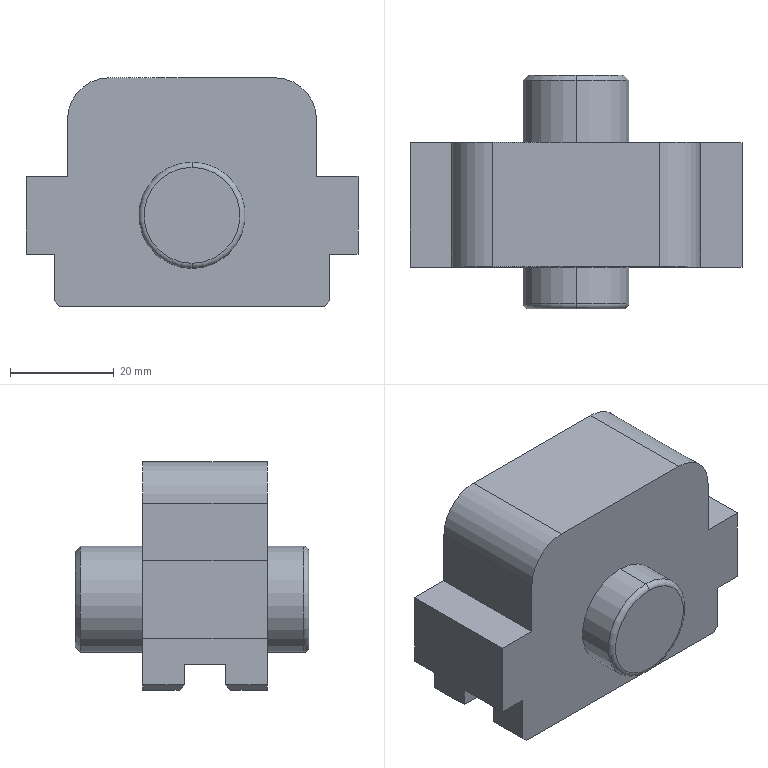Part | SolidWorks | features ICE 5, Chamfer 2, CutThin 1, Draft 1, Extrusion 1, Fillet 1 | 1 solid | 56 faces | box 64 x 45 x 44 mm | volume 54258 mm3 | plane 32 | cylinder 18 | cone 4 | torus 2 | commonest cylinder face diameters 3 x4 6 x4 20.5 x4 13 x2 16 x2 17 x2
STEP:
#1=CARTESIAN_POINT('',(0.,37.,-17.25));
#2=VERTEX_POINT('',#1);
#3=CARTESIAN_POINT('',(0.,37.,-35.75));
#4=VERTEX_POINT('',#3);
#5=CARTESIAN_POINT('',(0.,37.,-26.5));
#6=DIRECTION('',(0.,1.,0.));
#7=DIRECTION('',(0.,0.,1.));
#8=AXIS2_PLACEMENT_3D('',#5,#6,#7);
#9=CIRCLE('',#8,9.25);
#10=EDGE_CURVE('',#2,#4,#9,.T.);
#11=ORIENTED_EDGE('',*,*,#10,.F.);
#12=CARTESIAN_POINT('',(0.,36.,-16.25));
#13=VERTEX_POINT('',#12);
#14=CARTESIAN_POINT('',(0.,37.,-17.25));
#15=DIRECTION('',(0.,-0.7071,0.7071));
#16=VECTOR('',#15,1000.);
#17=LINE('',#14,#16);
#18=EDGE_CURVE('',#2,#13,#17,.T.);
#19=ORIENTED_EDGE('',*,*,#18,.T.);
#20=CARTESIAN_POINT('',(0.,36.,-36.75));
#21=VERTEX_POINT('',#20);
#22=CARTESIAN_POINT('',(0.,36.,-26.5));
#23=DIRECTION('',(0.,-1.,0.));
#24=DIRECTION('',(0.,0.,1.));
#25=AXIS2_PLACEMENT_3D('',#22,#23,#24);
#26=CIRCLE('',#25,10.25);
#27=EDGE_CURVE('',#21,#13,#26,.T.);
#28=ORIENTED_EDGE('',*,*,#27,.F.);
#29=CARTESIAN_POINT('',(0.,37.,-35.75));
#30=DIRECTION('',(0.,-0.7071,-0.7071));
#31=VECTOR('',#30,1000.);
#32=LINE('',#29,#31);
#33=EDGE_CURVE('',#4,#21,#32,.T.);
#34=ORIENTED_EDGE('',*,*,#33,.F.);
#35=EDGE_LOOP('',(#11,#19,#28,#34));
#36=FACE_OUTER_BOUND('',#35,.T.);
#37=CARTESIAN_POINT('',(0.,37.,-26.5));
#38=DIRECTION('',(0.,-1.,0.));
#39=DIRECTION('',(0.,0.,-1.));
#40=AXIS2_PLACEMENT_3D('',#37,#38,#39);
#41=CONICAL_SURFACE('',#40,9.25,0.7854);
#42=ADVANCED_FACE('',(#36),#41,.T.);
#43=CARTESIAN_POINT('',(0.,-3.,-33.));
#44=VERTEX_POINT('',#43);
#45=CARTESIAN_POINT('',(0.,-3.,-20.));
#46=VERTEX_POINT('',#45);
#47=CARTESIAN_POINT('',(0.,-3.,-26.5));
#48=DIRECTION('',(0.,1.,0.));
#49=DIRECTION('',(0.,0.,1.));
#50=AXIS2_PLACEMENT_3D('',#47,#48,#49);
#51=CIRCLE('',#50,6.5);
#52=EDGE_CURVE('',#44,#46,#51,.T.);
#53=ORIENTED_EDGE('',*,*,#52,.F.);
#54=CARTESIAN_POINT('',(0.,37.,-33.));
#55=VERTEX_POINT('',#54);
#56=CARTESIAN_POINT('',(0.,-3.,-33.));
#57=DIRECTION('',(0.,1.,0.));
#58=VECTOR('',#57,1000.);
#59=LINE('',#56,#58);
#60=EDGE_CURVE('',#44,#55,#59,.T.);
#61=ORIENTED_EDGE('',*,*,#60,.T.);
#62=CARTESIAN_POINT('',(0.,37.,-20.));
#63=VERTEX_POINT('',#62);
#64=CARTESIAN_POINT('',(0.,37.,-26.5));
#65=DIRECTION('',(0.,1.,0.));
#66=DIRECTION('',(0.,0.,1.));
#67=AXIS2_PLACEMENT_3D('',#64,#65,#66);
#68=CIRCLE('',#67,6.5);
#69=EDGE_CURVE('',#55,#63,#68,.T.);
#70=ORIENTED_EDGE('',*,*,#69,.T.);
#71=CARTESIAN_POINT('',(0.,-3.,-20.));
#72=DIRECTION('',(0.,1.,0.));
#73=VECTOR('',#72,1000.);
#74=LINE('',#71,#73);
#75=EDGE_CURVE('',#46,#63,#74,.T.);
#76=ORIENTED_EDGE('',*,*,#75,.F.);
#77=EDGE_LOOP('',(#53,#61,#70,#76));
#78=FACE_OUTER_BOUND('',#77,.T.);
#79=CARTESIAN_POINT('',(0.,-3.,-26.5));
#80=DIRECTION('',(0.,1.,0.));
#81=DIRECTION('',(0.,0.,1.));
#82=AXIS2_PLACEMENT_3D('',#79,#80,#81);
#83=CYLINDRICAL_SURFACE('',#82,6.5);
#84=ADVANCED_FACE('',(#78),#83,.F.);
#85=CARTESIAN_POINT('',(0.,34.253,-35.));
#86=VERTEX_POINT('',#85);
#87=CARTESIAN_POINT('',(-8.5,34.253,-26.5));
#88=VERTEX_POINT('',#87);
#89=CARTESIAN_POINT('',(0.,34.253,-26.5));
#90=DIRECTION('',(0.,1.,0.));
#91=DIRECTION('',(0.,0.,-1.));
#92=AXIS2_PLACEMENT_3D('',#89,#90,#91);
#93=CIRCLE('',#92,8.5);
#94=EDGE_CURVE('',#86,#88,#93,.T.);
#95=ORIENTED_EDGE('',*,*,#94,.F.);
#96=CARTESIAN_POINT('',(0.,37.,-35.));
#97=VERTEX_POINT('',#96);
#98=CARTESIAN_POINT('',(0.,34.,-35.));
#99=DIRECTION('',(0.,1.,0.));
#100=VECTOR('',#99,1000.);
#101=LINE('',#98,#100);
#102=EDGE_CURVE('',#86,#97,#101,.T.);
#103=ORIENTED_EDGE('',*,*,#102,.T.);
#104=CARTESIAN_POINT('',(0.,37.,-18.));
#105=VERTEX_POINT('',#104);
#106=CARTESIAN_POINT('',(0.,37.,-26.5));
#107=DIRECTION('',(0.,1.,0.));
#108=DIRECTION('',(1.,0.,0.));
#109=AXIS2_PLACEMENT_3D('',#106,#107,#108);
#110=CIRCLE('',#109,8.5);
#111=EDGE_CURVE('',#97,#105,#110,.T.);
#112=ORIENTED_EDGE('',*,*,#111,.T.);
#113=CARTESIAN_POINT('',(0.,34.253,-18.));
#114=VERTEX_POINT('',#113);
#115=CARTESIAN_POINT('',(0.,34.,-18.));
#116=DIRECTION('',(0.,1.,0.));
#117=VECTOR('',#116,1000.);
#118=LINE('',#115,#117);
#119=EDGE_CURVE('',#114,#105,#118,.T.);
#120=ORIENTED_EDGE('',*,*,#119,.F.);
#121=CARTESIAN_POINT('',(0.,34.253,-26.5));
#122=DIRECTION('',(0.,1.,0.));
#123=DIRECTION('',(0.,0.,-1.));
#124=AXIS2_PLACEMENT_3D('',#121,#122,#123);
#125=CIRCLE('',#124,8.5);
#126=EDGE_CURVE('',#88,#114,#125,.T.);
#127=ORIENTED_EDGE('',*,*,#126,.F.);
#128=EDGE_LOOP('',(#95,#103,#112,#120,#127));
#129=FACE_OUTER_BOUND('',#128,.T.);
#130=CARTESIAN_POINT('',(0.,34.,-26.5));
#131=DIRECTION('',(0.,1.,0.));
#132=DIRECTION('',(0.,0.,1.));
#133=AXIS2_PLACEMENT_3D('',#130,#131,#132);
#134=CYLINDRICAL_SURFACE('',#133,8.5);
#135=ADVANCED_FACE('',(#129),#134,.F.);
#136=CARTESIAN_POINT('',(1.5,18.5,-39.));
#137=VERTEX_POINT('',#136);
#138=CARTESIAN_POINT('',(-1.5,18.5,-39.));
#139=VERTEX_POINT('',#138);
#140=CARTESIAN_POINT('',(0.,18.5,-39.));
#141=DIRECTION('',(0.,0.,-1.));
#142=DIRECTION('',(-1.,0.,0.));
#143=AXIS2_PLACEMENT_3D('',#140,#141,#142);
#144=CIRCLE('',#143,1.5);
#145=EDGE_CURVE('',#137,#139,#144,.T.);
#146=ORIENTED_EDGE('',*,*,#145,.F.);
#147=CARTESIAN_POINT('',(1.5,18.5,-44.));
#148=VERTEX_POINT('',#147);
#149=CARTESIAN_POINT('',(1.5,18.5,-39.));
#150=DIRECTION('',(0.,0.,-1.));
#151=VECTOR('',#150,1000.);
#152=LINE('',#149,#151);
#153=EDGE_CURVE('',#137,#148,#152,.T.);
#154=ORIENTED_EDGE('',*,*,#153,.T.);
#155=CARTESIAN_POINT('',(0.,17.,-44.));
#156=VERTEX_POINT('',#155);
#157=CARTESIAN_POINT('',(0.,18.5,-44.));
#158=DIRECTION('',(0.,0.,-1.));
#159=DIRECTION('',(-1.,0.,0.));
#160=AXIS2_PLACEMENT_3D('',#157,#158,#159);
#161=CIRCLE('',#160,1.5);
#162=EDGE_CURVE('',#148,#156,#161,.T.);
#163=ORIENTED_EDGE('',*,*,#162,.T.);
#164=CARTESIAN_POINT('',(-1.5,18.5,-44.));
#165=VERTEX_POINT('',#164);
#166=CARTESIAN_POINT('',(0.,18.5,-44.));
#167=DIRECTION('',(0.,0.,-1.));
#168=DIRECTION('',(-1.,0.,0.));
#169=AXIS2_PLACEMENT_3D('',#166,#167,#168);
#170=CIRCLE('',#169,1.5);
#171=EDGE_CURVE('',#156,#165,#170,.T.);
#172=ORIENTED_EDGE('',*,*,#171,.T.);
#173=CARTESIAN_POINT('',(-1.5,18.5,-39.));
#174=DIRECTION('',(0.,0.,-1.));
#175=VECTOR('',#174,1000.);
#176=LINE('',#173,#175);
#177=EDGE_CURVE('',#139,#165,#176,.T.);
#178=ORIENTED_EDGE('',*,*,#177,.F.);
#179=EDGE_LOOP('',(#146,#154,#163,#172,#178));
#180=FACE_OUTER_BOUND('',#179,.T.);
#181=CARTESIAN_POINT('',(0.,18.5,-39.));
#182=DIRECTION('',(0.,0.,-1.));
#183=DIRECTION('',(-1.,0.,0.));
#184=AXIS2_PLACEMENT_3D('',#181,#182,#183);
#185=CYLINDRICAL_SURFACE('',#184,1.5);
#186=ADVANCED_FACE('',(#180),#185,.F.);
#187=CARTESIAN_POINT('',(1.5,5.5,-39.));
#188=VERTEX_POINT('',#187);
#189=CARTESIAN_POINT('',(-1.5,5.5,-39.));
#190=VERTEX_POINT('',#189);
#191=CARTESIAN_POINT('',(0.,5.5,-39.));
#192=DIRECTION('',(0.,0.,-1.));
#193=DIRECTION('',(1.,0.,0.));
#194=AXIS2_PLACEMENT_3D('',#191,#192,#193);
#195=CIRCLE('',#194,1.5);
#196=EDGE_CURVE('',#188,#190,#195,.T.);
#197=ORIENTED_EDGE('',*,*,#196,.F.);
#198=CARTESIAN_POINT('',(1.5,5.5,-44.));
#199=VERTEX_POINT('',#198);
#200=CARTESIAN_POINT('',(1.5,5.5,-39.));
#201=DIRECTION('',(0.,0.,-1.));
#202=VECTOR('',#201,1000.);
#203=LINE('',#200,#202);
#204=EDGE_CURVE('',#188,#199,#203,.T.);
#205=ORIENTED_EDGE('',*,*,#204,.T.);
#206=CARTESIAN_POINT('',(-1.5,5.5,-44.));
#207=VERTEX_POINT('',#206);
#208=CARTESIAN_POINT('',(0.,5.5,-44.));
#209=DIRECTION('',(0.,0.,-1.));
#210=DIRECTION('',(1.,0.,0.));
#211=AXIS2_PLACEMENT_3D('',#208,#209,#210);
#212=CIRCLE('',#211,1.5);
#213=EDGE_CURVE('',#199,#207,#212,.T.);
#214=ORIENTED_EDGE('',*,*,#213,.T.);
#215=CARTESIAN_POINT('',(-1.5,5.5,-39.));
#216=DIRECTION('',(0.,0.,-1.));
#217=VECTOR('',#216,1000.);
#218=LINE('',#215,#217);
#219=EDGE_CURVE('',#190,#207,#218,.T.);
#220=ORIENTED_EDGE('',*,*,#219,.F.);
#221=EDGE_LOOP('',(#197,#205,#214,#220));
#222=FACE_OUTER_BOUND('',#221,.T.);
#223=CARTESIAN_POINT('',(0.,5.5,-39.));
#224=DIRECTION('',(0.,0.,-1.));
#225=DIRECTION('',(-1.,0.,0.));
#226=AXIS2_PLACEMENT_3D('',#223,#224,#225);
#227=CYLINDRICAL_SURFACE('',#226,1.5);
#228=ADVANCED_FACE('',(#222),#227,.F.);
#229=CARTESIAN_POINT('',(19.5,12.,-4.));
#230=VERTEX_POINT('',#229);
#231=CARTESIAN_POINT('',(13.5,12.,-4.));
#232=VERTEX_POINT('',#231);
#233=CARTESIAN_POINT('',(16.5,12.,-4.));
#234=DIRECTION('',(0.,0.,-1.));
#235=DIRECTION('',(-1.,0.,0.));
#236=AXIS2_PLACEMENT_3D('',#233,#234,#235);
#237=CIRCLE('',#236,3.);
#238=EDGE_CURVE('',#230,#232,#237,.T.);
#239=ORIENTED_EDGE('',*,*,#238,.F.);
#240=CARTESIAN_POINT('',(19.5,12.,-39.));
#241=VERTEX_POINT('',#240);
#242=CARTESIAN_POINT('',(19.5,12.,-4.));
#243=DIRECTION('',(0.,0.,-1.));
#244=VECTOR('',#243,1000.);
#245=LINE('',#242,#244);
#246=EDGE_CURVE('',#230,#241,#245,.T.);
#247=ORIENTED_EDGE('',*,*,#246,.T.);
#248=CARTESIAN_POINT('',(13.5,12.,-39.));
#249=VERTEX_POINT('',#248);
#250=CARTESIAN_POINT('',(16.5,12.,-39.));
#251=DIRECTION('',(0.,0.,-1.));
#252=DIRECTION('',(-1.,0.,0.));
#253=AXIS2_PLACEMENT_3D('',#250,#251,#252);
#254=CIRCLE('',#253,3.);
#255=EDGE_CURVE('',#241,#249,#254,.T.);
#256=ORIENTED_EDGE('',*,*,#255,.T.);
#257=CARTESIAN_POINT('',(13.5,12.,-4.));
#258=DIRECTION('',(0.,0.,-1.));
#259=VECTOR('',#258,1000.);
#260=LINE('',#257,#259);
#261=EDGE_CURVE('',#232,#249,#260,.T.);
#262=ORIENTED_EDGE('',*,*,#261,.F.);
#263=EDGE_LOOP('',(#239,#247,#256,#262));
#264=FACE_OUTER_BOUND('',#263,.T.);
#265=CARTESIAN_POINT('',(16.5,12.,-4.));
#266=DIRECTION('',(0.,0.,-1.));
#267=DIRECTION('',(-1.,0.,0.));
#268=AXIS2_PLACEMENT_3D('',#265,#266,#267);
#269=CYLINDRICAL_SURFACE('',#268,3.);
#270=ADVANCED_FACE('',(#264),#269,.F.);
#271=CARTESIAN_POINT('',(-13.5,12.,-4.));
#272=VERTEX_POINT('',#271);
#273=CARTESIAN_POINT('',(-19.5,12.,-4.));
#274=VERTEX_POINT('',#273);
#275=CARTESIAN_POINT('',(-16.5,12.,-4.));
#276=DIRECTION('',(0.,0.,-1.));
#277=DIRECTION('',(1.,0.,0.));
#278=AXIS2_PLACEMENT_3D('',#275,#276,#277);
#279=CIRCLE('',#278,3.);
#280=EDGE_CURVE('',#272,#274,#279,.T.);
#281=ORIENTED_EDGE('',*,*,#280,.F.);
#282=CARTESIAN_POINT('',(-13.5,12.,-39.));
#283=VERTEX_POINT('',#282);
#284=CARTESIAN_POINT('',(-13.5,12.,-4.));
#285=DIRECTION('',(0.,0.,-1.));
#286=VECTOR('',#285,1000.);
#287=LINE('',#284,#286);
#288=EDGE_CURVE('',#272,#283,#287,.T.);
#289=ORIENTED_EDGE('',*,*,#288,.T.);
#290=CARTESIAN_POINT('',(-19.5,12.,-39.));
#291=VERTEX_POINT('',#290);
#292=CARTESIAN_POINT('',(-16.5,12.,-39.));
#293=DIRECTION('',(0.,0.,-1.));
#294=DIRECTION('',(1.,0.,0.));
#295=AXIS2_PLACEMENT_3D('',#292,#293,#294);
#296=CIRCLE('',#295,3.);
#297=EDGE_CURVE('',#283,#291,#296,.T.);
#298=ORIENTED_EDGE('',*,*,#297,.T.);
#299=CARTESIAN_POINT('',(-19.5,12.,-4.));
#300=DIRECTION('',(0.,0.,-1.));
#301=VECTOR('',#300,1000.);
#302=LINE('',#299,#301);
#303=EDGE_CURVE('',#274,#291,#302,.T.);
#304=ORIENTED_EDGE('',*,*,#303,.F.);
#305=EDGE_LOOP('',(#281,#289,#298,#304));
#306=FACE_OUTER_BOUND('',#305,.T.);
#307=CARTESIAN_POINT('',(-16.5,12.,-4.));
#308=DIRECTION('',(0.,0.,-1.));
#309=DIRECTION('',(-1.,0.,0.));
#310=AXIS2_PLACEMENT_3D('',#307,#308,#309);
#311=CYLINDRICAL_SURFACE('',#310,3.);
#312=ADVANCED_FACE('',(#306),#311,.F.);
#313=CARTESIAN_POINT('',(0.,-8.,-35.75));
#314=VERTEX_POINT('',#313);
#315=CARTESIAN_POINT('',(0.,-8.,-17.25));
#316=VERTEX_POINT('',#315);
#317=CARTESIAN_POINT('',(0.,-8.,-26.5));
#318=DIRECTION('',(0.,-1.,0.));
#319=DIRECTION('',(0.,0.,1.));
#320=AXIS2_PLACEMENT_3D('',#317,#318,#319);
#321=CIRCLE('',#320,9.25);
#322=EDGE_CURVE('',#314,#316,#321,.T.);
#323=ORIENTED_EDGE('',*,*,#322,.F.);
#324=CARTESIAN_POINT('',(0.,-7.,-36.75));
#325=VERTEX_POINT('',#324);
#326=CARTESIAN_POINT('',(0.,-7.,-35.75));
#327=DIRECTION('',(1.,0.,0.));
#328=DIRECTION('',(0.,0.,-1.));
#329=AXIS2_PLACEMENT_3D('',#326,#327,#328);
#330=CIRCLE('',#329,1.);
#331=EDGE_CURVE('',#314,#325,#330,.T.);
#332=ORIENTED_EDGE('',*,*,#331,.T.);
#333=CARTESIAN_POINT('',(0.,-7.,-16.25));
#334=VERTEX_POINT('',#333);
#335=CARTESIAN_POINT('',(0.,-7.,-26.5));
#336=DIRECTION('',(0.,1.,0.));
#337=DIRECTION('',(0.,0.,1.));
#338=AXIS2_PLACEMENT_3D('',#335,#336,#337);
#339=CIRCLE('',#338,10.25);
#340=EDGE_CURVE('',#334,#325,#339,.T.);
#341=ORIENTED_EDGE('',*,*,#340,.F.);
#342=CARTESIAN_POINT('',(0.,-7.,-17.25));
#343=DIRECTION('',(-1.,0.,0.));
#344=DIRECTION('',(0.,0.,1.));
#345=AXIS2_PLACEMENT_3D('',#342,#343,#344);
#346=CIRCLE('',#345,1.);
#347=EDGE_CURVE('',#316,#334,#346,.T.);
#348=ORIENTED_EDGE('',*,*,#347,.F.);
#349=EDGE_LOOP('',(#323,#332,#341,#348));
#350=FACE_OUTER_BOUND('',#349,.T.);
#351=CARTESIAN_POINT('',(0.,-7.,-26.5));
#352=DIRECTION('',(0.,1.,0.));
#353=DIRECTION('',(0.,0.,1.));
#354=AXIS2_PLACEMENT_3D('',#351,#352,#353);
#355=TOROIDAL_SURFACE('',#354,9.25,1.);
#356=ADVANCED_FACE('',(#350),#355,.T.);
#357=ORIENTED_EDGE('',*,*,#27,.T.);
#358=CARTESIAN_POINT('',(0.,24.,-16.25));
#359=VERTEX_POINT('',#358);
#360=CARTESIAN_POINT('',(0.,37.,-16.25));
#361=DIRECTION('',(0.,-1.,0.));
#362=VECTOR('',#361,1000.);
#363=LINE('',#360,#362);
#364=EDGE_CURVE('',#13,#359,#363,.T.);
#365=ORIENTED_EDGE('',*,*,#364,.T.);
#366=CARTESIAN_POINT('',(0.,24.,-36.75));
#367=VERTEX_POINT('',#366);
#368=CARTESIAN_POINT('',(0.,24.,-26.5));
#369=DIRECTION('',(0.,1.,0.));
#370=DIRECTION('',(0.,0.,-1.));
#371=AXIS2_PLACEMENT_3D('',#368,#369,#370);
#372=CIRCLE('',#371,10.25);
#373=EDGE_CURVE('',#359,#367,#372,.T.);
#374=ORIENTED_EDGE('',*,*,#373,.T.);
#375=CARTESIAN_POINT('',(0.,37.,-36.75));
#376=DIRECTION('',(0.,-1.,0.));
#377=VECTOR('',#376,1000.);
#378=LINE('',#375,#377);
#379=EDGE_CURVE('',#21,#367,#378,.T.);
#380=ORIENTED_EDGE('',*,*,#379,.F.);
#381=EDGE_LOOP('',(#357,#365,#374,#380));
#382=FACE_OUTER_BOUND('',#381,.T.);
#383=CARTESIAN_POINT('',(0.,37.,-26.5));
#384=DIRECTION('',(0.,-1.,0.));
#385=DIRECTION('',(0.,0.,-1.));
#386=AXIS2_PLACEMENT_3D('',#383,#384,#385);
#387=CYLINDRICAL_SURFACE('',#386,10.25);
#388=ADVANCED_FACE('',(#382),#387,.T.);
#389=CARTESIAN_POINT('',(0.,0.,-16.25));
#390=VERTEX_POINT('',#389);
#391=CARTESIAN_POINT('',(0.,0.,-36.75));
#392=VERTEX_POINT('',#391);
#393=CARTESIAN_POINT('',(0.,0.,-26.5));
#394=DIRECTION('',(0.,1.,0.));
#395=DIRECTION('',(0.,0.,-1.));
#396=AXIS2_PLACEMENT_3D('',#393,#394,#395);
#397=CIRCLE('',#396,10.25);
#398=EDGE_CURVE('',#390,#392,#397,.T.);
#399=ORIENTED_EDGE('',*,*,#398,.F.);
#400=CARTESIAN_POINT('',(0.,37.,-16.25));
#401=DIRECTION('',(0.,-1.,0.));
#402=VECTOR('',#401,1000.);
#403=LINE('',#400,#402);
#404=EDGE_CURVE('',#390,#334,#403,.T.);
#405=ORIENTED_EDGE('',*,*,#404,.T.);
#406=ORIENTED_EDGE('',*,*,#340,.T.);
#407=CARTESIAN_POINT('',(0.,37.,-36.75));
#408=DIRECTION('',(0.,-1.,0.));
#409=VECTOR('',#408,1000.);
#410=LINE('',#407,#409);
#411=EDGE_CURVE('',#392,#325,#410,.T.);
#412=ORIENTED_EDGE('',*,*,#411,.F.);
#413=EDGE_LOOP('',(#399,#405,#406,#412));
#414=FACE_OUTER_BOUND('',#413,.T.);
#415=CARTESIAN_POINT('',(0.,37.,-26.5));
#416=DIRECTION('',(0.,-1.,0.));
#417=DIRECTION('',(0.,0.,-1.));
#418=AXIS2_PLACEMENT_3D('',#415,#416,#417);
#419=CYLINDRICAL_SURFACE('',#418,10.25);
#420=ADVANCED_FACE('',(#414),#419,.T.);
#421=CARTESIAN_POINT('',(-7.5,37.,-26.5));
#422=VERTEX_POINT('',#421);
#423=CARTESIAN_POINT('',(7.5,37.,-26.5));
#424=VERTEX_POINT('',#423);
#425=CARTESIAN_POINT('',(0.,37.,-26.5));
#426=DIRECTION('',(0.,1.,0.));
#427=DIRECTION('',(1.,0.,0.));
#428=AXIS2_PLACEMENT_3D('',#425,#426,#427);
#429=CIRCLE('',#428,7.5);
#430=EDGE_CURVE('',#422,#424,#429,.T.);
#431=ORIENTED_EDGE('',*,*,#430,.F.);
#432=CARTESIAN_POINT('',(-7.5,37.,-26.5));
#433=DIRECTION('',(-0.342,-0.9397,0.));
#434=VECTOR('',#433,1000.);
#435=LINE('',#432,#434);
#436=EDGE_CURVE('',#422,#88,#435,.T.);
#437=ORIENTED_EDGE('',*,*,#436,.T.);
#438=ORIENTED_EDGE('',*,*,#126,.T.);
#439=CARTESIAN_POINT('',(8.5,34.253,-26.5));
#440=VERTEX_POINT('',#439);
#441=CARTESIAN_POINT('',(0.,34.253,-26.5));
#442=DIRECTION('',(0.,1.,0.));
#443=DIRECTION('',(0.,0.,-1.));
#444=AXIS2_PLACEMENT_3D('',#441,#442,#443);
#445=CIRCLE('',#444,8.5);
#446=EDGE_CURVE('',#114,#440,#445,.T.);
#447=ORIENTED_EDGE('',*,*,#446,.T.);
#448=CARTESIAN_POINT('',(7.5,37.,-26.5));
#449=DIRECTION('',(0.342,-0.9397,0.));
#450=VECTOR('',#449,1000.);
#451=LINE('',#448,#450);
#452=EDGE_CURVE('',#424,#440,#451,.T.);
#453=ORIENTED_EDGE('',*,*,#452,.F.);
#454=EDGE_LOOP('',(#431,#437,#438,#447,#453));
#455=FACE_OUTER_BOUND('',#454,.T.);
#456=CARTESIAN_POINT('',(0.,37.,-26.5));
#457=DIRECTION('',(0.,-1.,0.));
#458=DIRECTION('',(1.,0.,0.));
#459=AXIS2_PLACEMENT_3D('',#456,#457,#458);
#460=CONICAL_SURFACE('',#459,7.5,0.3491);
#461=ADVANCED_FACE('',(#455),#460,.T.);
#462=ORIENTED_EDGE('',*,*,#436,.F.);
#463=CARTESIAN_POINT('',(0.,37.,-26.5));
#464=DIRECTION('',(0.,1.,0.));
#465=DIRECTION('',(1.,0.,0.));
#466=AXIS2_PLACEMENT_3D('',#463,#464,#465);
#467=CIRCLE('',#466,7.5);
#468=EDGE_CURVE('',#424,#422,#467,.T.);
#469=ORIENTED_EDGE('',*,*,#468,.F.);
#470=ORIENTED_EDGE('',*,*,#452,.T.);
#471=CARTESIAN_POINT('',(0.,34.253,-26.5));
#472=DIRECTION('',(0.,1.,0.));
#473=DIRECTION('',(0.,0.,-1.));
#474=AXIS2_PLACEMENT_3D('',#471,#472,#473);
#475=CIRCLE('',#474,8.5);
#476=EDGE_CURVE('',#440,#86,#475,.T.);
#477=ORIENTED_EDGE('',*,*,#476,.T.);
#478=ORIENTED_EDGE('',*,*,#94,.T.);
#479=EDGE_LOOP('',(#462,#469,#470,#477,#478));
#480=FACE_OUTER_BOUND('',#479,.T.);
#481=CARTESIAN_POINT('',(0.,37.,-26.5));
#482=DIRECTION('',(0.,-1.,0.));
#483=DIRECTION('',(1.,0.,0.));
#484=AXIS2_PLACEMENT_3D('',#481,#482,#483);
#485=CONICAL_SURFACE('',#484,7.5,0.3491);
#486=ADVANCED_FACE('',(#480),#485,.T.);
#487=CARTESIAN_POINT('',(-25.5,17.,-44.));
#488=VERTEX_POINT('',#487);
#489=CARTESIAN_POINT('',(-26.5,17.,-44.));
#490=DIRECTION('',(-1.,0.,0.));
#491=VECTOR('',#490,1000.);
#492=LINE('',#489,#491);
#493=EDGE_CURVE('',#156,#488,#492,.T.);
#494=ORIENTED_EDGE('',*,*,#493,.T.);
#495=CARTESIAN_POINT('',(-25.5,24.,-44.));
#496=VERTEX_POINT('',#495);
#497=CARTESIAN_POINT('',(-25.5,24.,-44.));
#498=DIRECTION('',(0.,1.,0.));
#499=VECTOR('',#498,1000.);
#500=LINE('',#497,#499);
#501=EDGE_CURVE('',#488,#496,#500,.T.);
#502=ORIENTED_EDGE('',*,*,#501,.T.);
#503=CARTESIAN_POINT('',(25.5,24.,-44.));
#504=VERTEX_POINT('',#503);
#505=CARTESIAN_POINT('',(-26.5,24.,-44.));
#506=DIRECTION('',(-1.,0.,0.));
#507=VECTOR('',#506,1000.);
#508=LINE('',#505,#507);
#509=EDGE_CURVE('',#504,#496,#508,.T.);
#510=ORIENTED_EDGE('',*,*,#509,.F.);
#511=CARTESIAN_POINT('',(25.5,17.,-44.));
#512=VERTEX_POINT('',#511);
#513=CARTESIAN_POINT('',(25.5,24.,-44.));
#514=DIRECTION('',(0.,-1.,0.));
#515=VECTOR('',#514,1000.);
#516=LINE('',#513,#515);
#517=EDGE_CURVE('',#504,#512,#516,.T.);
#518=ORIENTED_EDGE('',*,*,#517,.T.);
#519=CARTESIAN_POINT('',(-26.5,17.,-44.));
#520=DIRECTION('',(-1.,0.,0.));
#521=VECTOR('',#520,1000.);
#522=LINE('',#519,#521);
#523=EDGE_CURVE('',#512,#156,#522,.T.);
#524=ORIENTED_EDGE('',*,*,#523,.T.);
#525=ORIENTED_EDGE('',*,*,#162,.F.);
#526=CARTESIAN_POINT('',(0.,18.5,-44.));
#527=DIRECTION('',(0.,0.,-1.));
#528=DIRECTION('',(-1.,0.,0.));
#529=AXIS2_PLACEMENT_3D('',#526,#527,#528);
#530=CIRCLE('',#529,1.5);
#531=EDGE_CURVE('',#165,#148,#530,.T.);
#532=ORIENTED_EDGE('',*,*,#531,.F.);
#533=ORIENTED_EDGE('',*,*,#171,.F.);
#534=EDGE_LOOP('',(#494,#502,#510,#518,#524,#525,#532,#533));
#535=FACE_OUTER_BOUND('',#534,.T.);
#536=CARTESIAN_POINT('',(-26.5,24.,-44.));
#537=DIRECTION('',(0.,0.,1.));
#538=DIRECTION('',(1.,0.,0.));
#539=AXIS2_PLACEMENT_3D('',#536,#537,#538);
#540=PLANE('',#539);
#541=ADVANCED_FACE('',(#535),#540,.F.);
#542=CARTESIAN_POINT('',(-24.,0.,-8.));
#543=VERTEX_POINT('',#542);
#544=CARTESIAN_POINT('',(-16.,0.,0.));
#545=VERTEX_POINT('',#544);
#546=CARTESIAN_POINT('',(-16.,0.,-8.));
#547=DIRECTION('',(0.,1.,0.));
#548=DIRECTION('',(0.,0.,-1.));
#549=AXIS2_PLACEMENT_3D('',#546,#547,#548);
#550=CIRCLE('',#549,8.);
#551=EDGE_CURVE('',#543,#545,#550,.T.);
#552=ORIENTED_EDGE('',*,*,#551,.T.);
#553=CARTESIAN_POINT('',(-16.,24.,0.));
#554=VERTEX_POINT('',#553);
#555=CARTESIAN_POINT('',(-16.,24.,0.));
#556=DIRECTION('',(0.,-1.,0.));
#557=VECTOR('',#556,1000.);
#558=LINE('',#555,#557);
#559=EDGE_CURVE('',#554,#545,#558,.T.);
#560=ORIENTED_EDGE('',*,*,#559,.F.);
#561=CARTESIAN_POINT('',(-24.,24.,-8.));
#562=VERTEX_POINT('',#561);
#563=CARTESIAN_POINT('',(-16.,24.,-8.));
#564=DIRECTION('',(0.,1.,0.));
#565=DIRECTION('',(0.,0.,-1.));
#566=AXIS2_PLACEMENT_3D('',#563,#564,#565);
#567=CIRCLE('',#566,8.);
#568=EDGE_CURVE('',#562,#554,#567,.T.);
#569=ORIENTED_EDGE('',*,*,#568,.F.);
#570=CARTESIAN_POINT('',(-24.,24.,-8.));
#571=DIRECTION('',(0.,-1.,0.));
#572=VECTOR('',#571,1000.);
#573=LINE('',#570,#572);
#574=EDGE_CURVE('',#562,#543,#573,.T.);
#575=ORIENTED_EDGE('',*,*,#574,.T.);
#576=EDGE_LOOP('',(#552,#560,#569,#575));
#577=FACE_OUTER_BOUND('',#576,.T.);
#578=CARTESIAN_POINT('',(-16.,24.,-8.));
#579=DIRECTION('',(0.,-1.,0.));
#580=DIRECTION('',(0.,0.,-1.));
#581=AXIS2_PLACEMENT_3D('',#578,#579,#580);
#582=CYLINDRICAL_SURFACE('',#581,8.);
#583=ADVANCED_FACE('',(#577),#582,.T.);
#584=CARTESIAN_POINT('',(16.,0.,0.));
#585=VERTEX_POINT('',#584);
#586=CARTESIAN_POINT('',(16.,0.,0.));
#587=DIRECTION('',(1.,0.,0.));
#588=VECTOR('',#587,1000.);
#589=LINE('',#586,#588);
#590=EDGE_CURVE('',#545,#585,#589,.T.);
#591=ORIENTED_EDGE('',*,*,#590,.T.);
#592=CARTESIAN_POINT('',(16.,24.,0.));
#593=VERTEX_POINT('',#592);
#594=CARTESIAN_POINT('',(16.,24.,0.));
#595=DIRECTION('',(0.,-1.,0.));
#596=VECTOR('',#595,1000.);
#597=LINE('',#594,#596);
#598=EDGE_CURVE('',#593,#585,#597,.T.);
#599=ORIENTED_EDGE('',*,*,#598,.F.);
#600=CARTESIAN_POINT('',(16.,24.,0.));
#601=DIRECTION('',(1.,0.,0.));
#602=VECTOR('',#601,1000.);
#603=LINE('',#600,#602);
#604=EDGE_CURVE('',#554,#593,#603,.T.);
#605=ORIENTED_EDGE('',*,*,#604,.F.);
#606=ORIENTED_EDGE('',*,*,#559,.T.);
#607=EDGE_LOOP('',(#591,#599,#605,#606));
#608=FACE_OUTER_BOUND('',#607,.T.);
#609=CARTESIAN_POINT('',(16.,24.,0.));
#610=DIRECTION('',(0.,0.,-1.));
#611=DIRECTION('',(-1.,0.,0.));
#612=AXIS2_PLACEMENT_3D('',#609,#610,#611);
#613=PLANE('',#612);
#614=ADVANCED_FACE('',(#608),#613,.F.);
#615=CARTESIAN_POINT('',(24.,0.,-8.));
#616=VERTEX_POINT('',#615);
#617=CARTESIAN_POINT('',(16.,0.,-8.));
#618=DIRECTION('',(0.,1.,0.));
#619=DIRECTION('',(0.,0.,1.));
#620=AXIS2_PLACEMENT_3D('',#617,#618,#619);
#621=CIRCLE('',#620,8.);
#622=EDGE_CURVE('',#585,#616,#621,.T.);
#623=ORIENTED_EDGE('',*,*,#622,.T.);
#624=CARTESIAN_POINT('',(24.,24.,-8.));
#625=VERTEX_POINT('',#624);
#626=CARTESIAN_POINT('',(24.,24.,-8.));
#627=DIRECTION('',(0.,-1.,0.));
#628=VECTOR('',#627,1000.);
#629=LINE('',#626,#628);
#630=EDGE_CURVE('',#625,#616,#629,.T.);
#631=ORIENTED_EDGE('',*,*,#630,.F.);
#632=CARTESIAN_POINT('',(16.,24.,-8.));
#633=DIRECTION('',(0.,1.,0.));
#634=DIRECTION('',(0.,0.,1.));
#635=AXIS2_PLACEMENT_3D('',#632,#633,#634);
#636=CIRCLE('',#635,8.);
#637=EDGE_CURVE('',#593,#625,#636,.T.);
#638=ORIENTED_EDGE('',*,*,#637,.F.);
#639=ORIENTED_EDGE('',*,*,#598,.T.);
#640=EDGE_LOOP('',(#623,#631,#638,#639));
#641=FACE_OUTER_BOUND('',#640,.T.);
#642=CARTESIAN_POINT('',(16.,24.,-8.));
#643=DIRECTION('',(0.,-1.,0.));
#644=DIRECTION('',(0.,0.,-1.));
#645=AXIS2_PLACEMENT_3D('',#642,#643,#644);
#646=CYLINDRICAL_SURFACE('',#645,8.);
#647=ADVANCED_FACE('',(#641),#646,.T.);
#648=CARTESIAN_POINT('',(24.,0.,-19.));
#649=VERTEX_POINT('',#648);
#650=CARTESIAN_POINT('',(24.,0.,-8.));
#651=DIRECTION('',(0.,0.,-1.));
#652=VECTOR('',#651,1000.);
#653=LINE('',#650,#652);
#654=EDGE_CURVE('',#616,#649,#653,.T.);
#655=ORIENTED_EDGE('',*,*,#654,.T.);
#656=CARTESIAN_POINT('',(24.,24.,-19.));
#657=VERTEX_POINT('',#656);
#658=CARTESIAN_POINT('',(24.,24.,-19.));
#659=DIRECTION('',(0.,-1.,0.));
#660=VECTOR('',#659,1000.);
#661=LINE('',#658,#660);
#662=EDGE_CURVE('',#657,#649,#661,.T.);
#663=ORIENTED_EDGE('',*,*,#662,.F.);
#664=CARTESIAN_POINT('',(24.,24.,-8.));
#665=DIRECTION('',(0.,0.,-1.));
#666=VECTOR('',#665,1000.);
#667=LINE('',#664,#666);
#668=EDGE_CURVE('',#625,#657,#667,.T.);
#669=ORIENTED_EDGE('',*,*,#668,.F.);
#670=ORIENTED_EDGE('',*,*,#630,.T.);
#671=EDGE_LOOP('',(#655,#663,#669,#670));
#672=FACE_OUTER_BOUND('',#671,.T.);
#673=CARTESIAN_POINT('',(24.,24.,-8.));
#674=DIRECTION('',(-1.,0.,0.));
#675=DIRECTION('',(0.,0.,1.));
#676=AXIS2_PLACEMENT_3D('',#673,#674,#675);
#677=PLANE('',#676);
#678=ADVANCED_FACE('',(#672),#677,.F.);
#679=CARTESIAN_POINT('',(32.,0.,-19.));
#680=VERTEX_POINT('',#679);
#681=CARTESIAN_POINT('',(24.,0.,-19.));
#682=DIRECTION('',(1.,0.,0.));
#683=VECTOR('',#682,1000.);
#684=LINE('',#681,#683);
#685=EDGE_CURVE('',#649,#680,#684,.T.);
#686=ORIENTED_EDGE('',*,*,#685,.T.);
#687=CARTESIAN_POINT('',(32.,24.,-19.));
#688=VERTEX_POINT('',#687);
#689=CARTESIAN_POINT('',(32.,24.,-19.));
#690=DIRECTION('',(0.,-1.,0.));
#691=VECTOR('',#690,1000.);
#692=LINE('',#689,#691);
#693=EDGE_CURVE('',#688,#680,#692,.T.);
#694=ORIENTED_EDGE('',*,*,#693,.F.);
#695=CARTESIAN_POINT('',(24.,24.,-19.));
#696=DIRECTION('',(1.,0.,0.));
#697=VECTOR('',#696,1000.);
#698=LINE('',#695,#697);
#699=EDGE_CURVE('',#657,#688,#698,.T.);
#700=ORIENTED_EDGE('',*,*,#699,.F.);
#701=ORIENTED_EDGE('',*,*,#662,.T.);
#702=EDGE_LOOP('',(#686,#694,#700,#701));
#703=FACE_OUTER_BOUND('',#702,.T.);
#704=CARTESIAN_POINT('',(24.,24.,-19.));
#705=DIRECTION('',(0.,0.,-1.));
#706=DIRECTION('',(-1.,0.,0.));
#707=AXIS2_PLACEMENT_3D('',#704,#705,#706);
#708=PLANE('',#707);
#709=ADVANCED_FACE('',(#703),#708,.F.);
#710=CARTESIAN_POINT('',(32.,0.,-34.));
#711=VERTEX_POINT('',#710);
#712=CARTESIAN_POINT('',(32.,0.,-19.));
#713=DIRECTION('',(0.,0.,-1.));
#714=VECTOR('',#713,1000.);
#715=LINE('',#712,#714);
#716=EDGE_CURVE('',#680,#711,#715,.T.);
#717=ORIENTED_EDGE('',*,*,#716,.T.);
#718=CARTESIAN_POINT('',(32.,24.,-34.));
#719=VERTEX_POINT('',#718);
#720=CARTESIAN_POINT('',(32.,24.,-34.));
#721=DIRECTION('',(0.,-1.,0.));
#722=VECTOR('',#721,1000.);
#723=LINE('',#720,#722);
#724=EDGE_CURVE('',#719,#711,#723,.T.);
#725=ORIENTED_EDGE('',*,*,#724,.F.);
#726=CARTESIAN_POINT('',(32.,24.,-19.));
#727=DIRECTION('',(0.,0.,-1.));
#728=VECTOR('',#727,1000.);
#729=LINE('',#726,#728);
#730=EDGE_CURVE('',#688,#719,#729,.T.);
#731=ORIENTED_EDGE('',*,*,#730,.F.);
#732=ORIENTED_EDGE('',*,*,#693,.T.);
#733=EDGE_LOOP('',(#717,#725,#731,#732));
#734=FACE_OUTER_BOUND('',#733,.T.);
#735=CARTESIAN_POINT('',(32.,24.,-19.));
#736=DIRECTION('',(-1.,0.,0.));
#737=DIRECTION('',(0.,0.,1.));
#738=AXIS2_PLACEMENT_3D('',#735,#736,#737);
#739=PLANE('',#738);
#740=ADVANCED_FACE('',(#734),#739,.F.);
#741=CARTESIAN_POINT('',(26.5,0.,-34.));
#742=VERTEX_POINT('',#741);
#743=CARTESIAN_POINT('',(32.,0.,-34.));
#744=DIRECTION('',(-1.,0.,0.));
#745=VECTOR('',#744,1000.);
#746=LINE('',#743,#745);
#747=EDGE_CURVE('',#711,#742,#746,.T.);
#748=ORIENTED_EDGE('',*,*,#747,.T.);
#749=CARTESIAN_POINT('',(26.5,24.,-34.));
#750=VERTEX_POINT('',#749);
#751=CARTESIAN_POINT('',(26.5,24.,-34.));
#752=DIRECTION('',(0.,-1.,0.));
#753=VECTOR('',#752,1000.);
#754=LINE('',#751,#753);
#755=EDGE_CURVE('',#750,#742,#754,.T.);
#756=ORIENTED_EDGE('',*,*,#755,.F.);
#757=CARTESIAN_POINT('',(32.,24.,-34.));
#758=DIRECTION('',(-1.,0.,0.));
#759=VECTOR('',#758,1000.);
#760=LINE('',#757,#759);
#761=EDGE_CURVE('',#719,#750,#760,.T.);
#762=ORIENTED_EDGE('',*,*,#761,.F.);
#763=ORIENTED_EDGE('',*,*,#724,.T.);
#764=EDGE_LOOP('',(#748,#756,#762,#763));
#765=FACE_OUTER_BOUND('',#764,.T.);
#766=CARTESIAN_POINT('',(32.,24.,-34.));
#767=DIRECTION('',(0.,0.,1.));
#768=DIRECTION('',(1.,0.,0.));
#769=AXIS2_PLACEMENT_3D('',#766,#767,#768);
#770=PLANE('',#769);
#771=ADVANCED_FACE('',(#765),#770,.F.);
#772=CARTESIAN_POINT('',(26.5,16.,-39.));
#773=VERTEX_POINT('',#772);
#774=CARTESIAN_POINT('',(26.5,16.,-43.));
#775=VERTEX_POINT('',#774);
#776=CARTESIAN_POINT('',(26.5,16.,-34.));
#777=DIRECTION('',(0.,0.,-1.));
#778=VECTOR('',#777,1000.);
#779=LINE('',#776,#778);
#780=EDGE_CURVE('',#773,#775,#779,.T.);
#781=ORIENTED_EDGE('',*,*,#780,.T.);
#782=CARTESIAN_POINT('',(26.5,24.,-43.));
#783=VERTEX_POINT('',#782);
#784=CARTESIAN_POINT('',(26.5,24.,-43.));
#785=DIRECTION('',(0.,1.,0.));
#786=VECTOR('',#785,1000.);
#787=LINE('',#784,#786);
#788=EDGE_CURVE('',#775,#783,#787,.T.);
#789=ORIENTED_EDGE('',*,*,#788,.T.);
#790=CARTESIAN_POINT('',(26.5,24.,-34.));
#791=DIRECTION('',(0.,0.,-1.));
#792=VECTOR('',#791,1000.);
#793=LINE('',#790,#792);
#794=EDGE_CURVE('',#750,#783,#793,.T.);
#795=ORIENTED_EDGE('',*,*,#794,.F.);
#796=ORIENTED_EDGE('',*,*,#755,.T.);
#797=CARTESIAN_POINT('',(26.5,0.,-43.));
#798=VERTEX_POINT('',#797);
#799=CARTESIAN_POINT('',(26.5,0.,-34.));
#800=DIRECTION('',(0.,0.,-1.));
#801=VECTOR('',#800,1000.);
#802=LINE('',#799,#801);
#803=EDGE_CURVE('',#742,#798,#802,.T.);
#804=ORIENTED_EDGE('',*,*,#803,.T.);
#805=CARTESIAN_POINT('',(26.5,8.,-43.));
#806=VERTEX_POINT('',#805);
#807=CARTESIAN_POINT('',(26.5,24.,-43.));
#808=DIRECTION('',(0.,1.,0.));
#809=VECTOR('',#808,1000.);
#810=LINE('',#807,#809);
#811=EDGE_CURVE('',#798,#806,#810,.T.);
#812=ORIENTED_EDGE('',*,*,#811,.T.);
#813=CARTESIAN_POINT('',(26.5,8.,-39.));
#814=VERTEX_POINT('',#813);
#815=CARTESIAN_POINT('',(26.5,8.,-34.));
#816=DIRECTION('',(0.,0.,1.));
#817=VECTOR('',#816,1000.);
#818=LINE('',#815,#817);
#819=EDGE_CURVE('',#806,#814,#818,.T.);
#820=ORIENTED_EDGE('',*,*,#819,.T.);
#821=CARTESIAN_POINT('',(26.5,24.,-39.));
#822=DIRECTION('',(0.,1.,0.));
#823=VECTOR('',#822,1000.);
#824=LINE('',#821,#823);
#825=EDGE_CURVE('',#814,#773,#824,.T.);
#826=ORIENTED_EDGE('',*,*,#825,.T.);
#827=EDGE_LOOP('',(#781,#789,#795,#796,#804,#812,#820,#826));
#828=FACE_OUTER_BOUND('',#827,.T.);
#829=CARTESIAN_POINT('',(26.5,24.,-34.));
#830=DIRECTION('',(-1.,0.,0.));
#831=DIRECTION('',(0.,0.,1.));
#832=AXIS2_PLACEMENT_3D('',#829,#830,#831);
#833=PLANE('',#832);
#834=ADVANCED_FACE('',(#828),#833,.F.);
#835=CARTESIAN_POINT('',(25.5,0.,-44.));
#836=VERTEX_POINT('',#835);
#837=CARTESIAN_POINT('',(-25.5,0.,-44.));
#838=VERTEX_POINT('',#837);
#839=CARTESIAN_POINT('',(-26.5,0.,-44.));
#840=DIRECTION('',(-1.,0.,0.));
#841=VECTOR('',#840,1000.);
#842=LINE('',#839,#841);
#843=EDGE_CURVE('',#836,#838,#842,.T.);
#844=ORIENTED_EDGE('',*,*,#843,.T.);
#845=CARTESIAN_POINT('',(-25.5,7.,-44.));
#846=VERTEX_POINT('',#845);
#847=CARTESIAN_POINT('',(-25.5,24.,-44.));
#848=DIRECTION('',(0.,1.,0.));
#849=VECTOR('',#848,1000.);
#850=LINE('',#847,#849);
#851=EDGE_CURVE('',#838,#846,#850,.T.);
#852=ORIENTED_EDGE('',*,*,#851,.T.);
#853=CARTESIAN_POINT('',(0.,7.,-44.));
#854=VERTEX_POINT('',#853);
#855=CARTESIAN_POINT('',(-26.5,7.,-44.));
#856=DIRECTION('',(1.,0.,0.));
#857=VECTOR('',#856,1000.);
#858=LINE('',#855,#857);
#859=EDGE_CURVE('',#846,#854,#858,.T.);
#860=ORIENTED_EDGE('',*,*,#859,.T.);
#861=CARTESIAN_POINT('',(0.,5.5,-44.));
#862=DIRECTION('',(0.,0.,-1.));
#863=DIRECTION('',(1.,0.,0.));
#864=AXIS2_PLACEMENT_3D('',#861,#862,#863);
#865=CIRCLE('',#864,1.5);
#866=EDGE_CURVE('',#207,#854,#865,.T.);
#867=ORIENTED_EDGE('',*,*,#866,.F.);
#868=ORIENTED_EDGE('',*,*,#213,.F.);
#869=CARTESIAN_POINT('',(0.,5.5,-44.));
#870=DIRECTION('',(0.,0.,-1.));
#871=DIRECTION('',(1.,0.,0.));
#872=AXIS2_PLACEMENT_3D('',#869,#870,#871);
#873=CIRCLE('',#872,1.5);
#874=EDGE_CURVE('',#854,#199,#873,.T.);
#875=ORIENTED_EDGE('',*,*,#874,.F.);
#876=CARTESIAN_POINT('',(25.5,7.,-44.));
#877=VERTEX_POINT('',#876);
#878=CARTESIAN_POINT('',(-26.5,7.,-44.));
#879=DIRECTION('',(1.,0.,0.));
#880=VECTOR('',#879,1000.);
#881=LINE('',#878,#880);
#882=EDGE_CURVE('',#854,#877,#881,.T.);
#883=ORIENTED_EDGE('',*,*,#882,.T.);
#884=CARTESIAN_POINT('',(25.5,24.,-44.));
#885=DIRECTION('',(0.,-1.,0.));
#886=VECTOR('',#885,1000.);
#887=LINE('',#884,#886);
#888=EDGE_CURVE('',#877,#836,#887,.T.);
#889=ORIENTED_EDGE('',*,*,#888,.T.);
#890=EDGE_LOOP('',(#844,#852,#860,#867,#868,#875,#883,#889));
#891=FACE_OUTER_BOUND('',#890,.T.);
#892=CARTESIAN_POINT('',(-26.5,24.,-44.));
#893=DIRECTION('',(0.,0.,1.));
#894=DIRECTION('',(1.,0.,0.));
#895=AXIS2_PLACEMENT_3D('',#892,#893,#894);
#896=PLANE('',#895);
#897=ADVANCED_FACE('',(#891),#896,.F.);
#898=CARTESIAN_POINT('',(-26.5,24.,-43.));
#899=VERTEX_POINT('',#898);
#900=CARTESIAN_POINT('',(-26.5,24.,-34.));
#901=VERTEX_POINT('',#900);
#902=CARTESIAN_POINT('',(-26.5,24.,-34.));
#903=DIRECTION('',(0.,0.,1.));
#904=VECTOR('',#903,1000.);
#905=LINE('',#902,#904);
#906=EDGE_CURVE('',#899,#901,#905,.T.);
#907=ORIENTED_EDGE('',*,*,#906,.F.);
#908=CARTESIAN_POINT('',(-26.5,16.,-43.));
#909=VERTEX_POINT('',#908);
#910=CARTESIAN_POINT('',(-26.5,24.,-43.));
#911=DIRECTION('',(0.,-1.,0.));
#912=VECTOR('',#911,1000.);
#913=LINE('',#910,#912);
#914=EDGE_CURVE('',#899,#909,#913,.T.);
#915=ORIENTED_EDGE('',*,*,#914,.T.);
#916=CARTESIAN_POINT('',(-26.5,16.,-39.));
#917=VERTEX_POINT('',#916);
#918=CARTESIAN_POINT('',(-26.5,16.,-39.));
#919=DIRECTION('',(0.,0.,-1.));
#920=VECTOR('',#919,1000.);
#921=LINE('',#918,#920);
#922=EDGE_CURVE('',#917,#909,#921,.T.);
#923=ORIENTED_EDGE('',*,*,#922,.F.);
#924=CARTESIAN_POINT('',(-26.5,8.,-39.));
#925=VERTEX_POINT('',#924);
#926=CARTESIAN_POINT('',(-26.5,8.,-39.));
#927=DIRECTION('',(0.,1.,0.));
#928=VECTOR('',#927,1000.);
#929=LINE('',#926,#928);
#930=EDGE_CURVE('',#925,#917,#929,.T.);
#931=ORIENTED_EDGE('',*,*,#930,.F.);
#932=CARTESIAN_POINT('',(-26.5,8.,-43.));
#933=VERTEX_POINT('',#932);
#934=CARTESIAN_POINT('',(-26.5,8.,-39.));
#935=DIRECTION('',(0.,0.,1.));
#936=VECTOR('',#935,1000.);
#937=LINE('',#934,#936);
#938=EDGE_CURVE('',#933,#925,#937,.T.);
#939=ORIENTED_EDGE('',*,*,#938,.F.);
#940=CARTESIAN_POINT('',(-26.5,0.,-43.));
#941=VERTEX_POINT('',#940);
#942=CARTESIAN_POINT('',(-26.5,24.,-43.));
#943=DIRECTION('',(0.,-1.,0.));
#944=VECTOR('',#943,1000.);
#945=LINE('',#942,#944);
#946=EDGE_CURVE('',#933,#941,#945,.T.);
#947=ORIENTED_EDGE('',*,*,#946,.T.);
#948=CARTESIAN_POINT('',(-26.5,0.,-34.));
#949=VERTEX_POINT('',#948);
#950=CARTESIAN_POINT('',(-26.5,0.,-34.));
#951=DIRECTION('',(0.,0.,1.));
#952=VECTOR('',#951,1000.);
#953=LINE('',#950,#952);
#954=EDGE_CURVE('',#941,#949,#953,.T.);
#955=ORIENTED_EDGE('',*,*,#954,.T.);
#956=CARTESIAN_POINT('',(-26.5,24.,-34.));
#957=DIRECTION('',(0.,-1.,0.));
#958=VECTOR('',#957,1000.);
#959=LINE('',#956,#958);
#960=EDGE_CURVE('',#901,#949,#959,.T.);
#961=ORIENTED_EDGE('',*,*,#960,.F.);
#962=EDGE_LOOP('',(#907,#915,#923,#931,#939,#947,#955,#961));
#963=FACE_OUTER_BOUND('',#962,.T.);
#964=CARTESIAN_POINT('',(-26.5,24.,-34.));
#965=DIRECTION('',(1.,0.,0.));
#966=DIRECTION('',(0.,0.,-1.));
#967=AXIS2_PLACEMENT_3D('',#964,#965,#966);
#968=PLANE('',#967);
#969=ADVANCED_FACE('',(#963),#968,.F.);
#970=CARTESIAN_POINT('',(-32.,0.,-34.));
#971=VERTEX_POINT('',#970);
#972=CARTESIAN_POINT('',(-32.,0.,-34.));
#973=DIRECTION('',(-1.,0.,0.));
#974=VECTOR('',#973,1000.);
#975=LINE('',#972,#974);
#976=EDGE_CURVE('',#949,#971,#975,.T.);
#977=ORIENTED_EDGE('',*,*,#976,.T.);
#978=CARTESIAN_POINT('',(-32.,24.,-34.));
#979=VERTEX_POINT('',#978);
#980=CARTESIAN_POINT('',(-32.,24.,-34.));
#981=DIRECTION('',(0.,-1.,0.));
#982=VECTOR('',#981,1000.);
#983=LINE('',#980,#982);
#984=EDGE_CURVE('',#979,#971,#983,.T.);
#985=ORIENTED_EDGE('',*,*,#984,.F.);
#986=CARTESIAN_POINT('',(-32.,24.,-34.));
#987=DIRECTION('',(-1.,0.,0.));
#988=VECTOR('',#987,1000.);
#989=LINE('',#986,#988);
#990=EDGE_CURVE('',#901,#979,#989,.T.);
#991=ORIENTED_EDGE('',*,*,#990,.F.);
#992=ORIENTED_EDGE('',*,*,#960,.T.);
#993=EDGE_LOOP('',(#977,#985,#991,#992));
#994=FACE_OUTER_BOUND('',#993,.T.);
#995=CARTESIAN_POINT('',(-32.,24.,-34.));
#996=DIRECTION('',(0.,0.,1.));
#997=DIRECTION('',(1.,0.,0.));
#998=AXIS2_PLACEMENT_3D('',#995,#996,#997);
#999=PLANE('',#998);
#1000=ADVANCED_FACE('',(#994),#999,.F.);
#1001=CARTESIAN_POINT('',(-32.,0.,-19.));
#1002=VERTEX_POINT('',#1001);
#1003=CARTESIAN_POINT('',(-32.,0.,-19.));
#1004=DIRECTION('',(0.,0.,1.));
#1005=VECTOR('',#1004,1000.);
#1006=LINE('',#1003,#1005);
#1007=EDGE_CURVE('',#971,#1002,#1006,.T.);
#1008=ORIENTED_EDGE('',*,*,#1007,.T.);
#1009=CARTESIAN_POINT('',(-32.,24.,-19.));
#1010=VERTEX_POINT('',#1009);
#1011=CARTESIAN_POINT('',(-32.,24.,-19.));
#1012=DIRECTION('',(0.,-1.,0.));
#1013=VECTOR('',#1012,1000.);
#1014=LINE('',#1011,#1013);
#1015=EDGE_CURVE('',#1010,#1002,#1014,.T.);
#1016=ORIENTED_EDGE('',*,*,#1015,.F.);
#1017=CARTESIAN_POINT('',(-32.,24.,-19.));
#1018=DIRECTION('',(0.,0.,1.));
#1019=VECTOR('',#1018,1000.);
#1020=LINE('',#1017,#1019);
#1021=EDGE_CURVE('',#979,#1010,#1020,.T.);
#1022=ORIENTED_EDGE('',*,*,#1021,.F.);
#1023=ORIENTED_EDGE('',*,*,#984,.T.);
#1024=EDGE_LOOP('',(#1008,#1016,#1022,#1023));
#1025=FACE_OUTER_BOUND('',#1024,.T.);
#1026=CARTESIAN_POINT('',(-32.,24.,-19.));
#1027=DIRECTION('',(1.,0.,0.));
#1028=DIRECTION('',(0.,0.,-1.));
#1029=AXIS2_PLACEMENT_3D('',#1026,#1027,#1028);
#1030=PLANE('',#1029);
#1031=ADVANCED_FACE('',(#1025),#1030,.F.);
#1032=CARTESIAN_POINT('',(-24.,0.,-19.));
#1033=VERTEX_POINT('',#1032);
#1034=CARTESIAN_POINT('',(-24.,0.,-19.));
#1035=DIRECTION('',(1.,0.,0.));
#1036=VECTOR('',#1035,1000.);
#1037=LINE('',#1034,#1036);
#1038=EDGE_CURVE('',#1002,#1033,#1037,.T.);
#1039=ORIENTED_EDGE('',*,*,#1038,.T.);
#1040=CARTESIAN_POINT('',(-24.,24.,-19.));
#1041=VERTEX_POINT('',#1040);
#1042=CARTESIAN_POINT('',(-24.,24.,-19.));
#1043=DIRECTION('',(0.,-1.,0.));
#1044=VECTOR('',#1043,1000.);
#1045=LINE('',#1042,#1044);
#1046=EDGE_CURVE('',#1041,#1033,#1045,.T.);
#1047=ORIENTED_EDGE('',*,*,#1046,.F.);
#1048=CARTESIAN_POINT('',(-24.,24.,-19.));
#1049=DIRECTION('',(1.,0.,0.));
#1050=VECTOR('',#1049,1000.);
#1051=LINE('',#1048,#1050);
#1052=EDGE_CURVE('',#1010,#1041,#1051,.T.);
#1053=ORIENTED_EDGE('',*,*,#1052,.F.);
#1054=ORIENTED_EDGE('',*,*,#1015,.T.);
#1055=EDGE_LOOP('',(#1039,#1047,#1053,#1054));
#1056=FACE_OUTER_BOUND('',#1055,.T.);
#1057=CARTESIAN_POINT('',(-24.,24.,-19.));
#1058=DIRECTION('',(0.,0.,-1.));
#1059=DIRECTION('',(-1.,0.,0.));
#1060=AXIS2_PLACEMENT_3D('',#1057,#1058,#1059);
#1061=PLANE('',#1060);
#1062=ADVANCED_FACE('',(#1056),#1061,.F.);
#1063=CARTESIAN_POINT('',(-24.,0.,-8.));
#1064=DIRECTION('',(0.,0.,1.));
#1065=VECTOR('',#1064,1000.);
#1066=LINE('',#1063,#1065);
#1067=EDGE_CURVE('',#1033,#543,#1066,.T.);
#1068=ORIENTED_EDGE('',*,*,#1067,.T.);
#1069=ORIENTED_EDGE('',*,*,#574,.F.);
#1070=CARTESIAN_POINT('',(-24.,24.,-8.));
#1071=DIRECTION('',(0.,0.,1.));
#1072=VECTOR('',#1071,1000.);
#1073=LINE('',#1070,#1072);
#1074=EDGE_CURVE('',#1041,#562,#1073,.T.);
#1075=ORIENTED_EDGE('',*,*,#1074,.F.);
#1076=ORIENTED_EDGE('',*,*,#1046,.T.);
#1077=EDGE_LOOP('',(#1068,#1069,#1075,#1076));
#1078=FACE_OUTER_BOUND('',#1077,.T.);
#1079=CARTESIAN_POINT('',(-24.,24.,-8.));
#1080=DIRECTION('',(1.,0.,0.));
#1081=DIRECTION('',(0.,0.,-1.));
#1082=AXIS2_PLACEMENT_3D('',#1079,#1080,#1081);
#1083=PLANE('',#1082);
#1084=ADVANCED_FACE('',(#1078),#1083,.F.);
#1085=CARTESIAN_POINT('',(0.,24.,-26.5));
#1086=DIRECTION('',(0.,1.,0.));
#1087=DIRECTION('',(0.,0.,-1.));
#1088=AXIS2_PLACEMENT_3D('',#1085,#1086,#1087);
#1089=CIRCLE('',#1088,10.25);
#1090=EDGE_CURVE('',#367,#359,#1089,.T.);
#1091=ORIENTED_EDGE('',*,*,#1090,.F.);
#1092=ORIENTED_EDGE('',*,*,#373,.F.);
#1093=EDGE_LOOP('',(#1091,#1092));
#1094=FACE_BOUND('',#1093,.T.);
#1095=ORIENTED_EDGE('',*,*,#509,.T.);
#1096=CARTESIAN_POINT('',(-26.5,24.,-43.));
#1097=DIRECTION('',(-0.7071,0.,0.7071));
#1098=VECTOR('',#1097,1000.);
#1099=LINE('',#1096,#1098);
#1100=EDGE_CURVE('',#496,#899,#1099,.T.);
#1101=ORIENTED_EDGE('',*,*,#1100,.T.);
#1102=ORIENTED_EDGE('',*,*,#906,.T.);
#1103=ORIENTED_EDGE('',*,*,#990,.T.);
#1104=ORIENTED_EDGE('',*,*,#1021,.T.);
#1105=ORIENTED_EDGE('',*,*,#1052,.T.);
#1106=ORIENTED_EDGE('',*,*,#1074,.T.);
#1107=ORIENTED_EDGE('',*,*,#568,.T.);
#1108=ORIENTED_EDGE('',*,*,#604,.T.);
#1109=ORIENTED_EDGE('',*,*,#637,.T.);
#1110=ORIENTED_EDGE('',*,*,#668,.T.);
#1111=ORIENTED_EDGE('',*,*,#699,.T.);
#1112=ORIENTED_EDGE('',*,*,#730,.T.);
#1113=ORIENTED_EDGE('',*,*,#761,.T.);
#1114=ORIENTED_EDGE('',*,*,#794,.T.);
#1115=CARTESIAN_POINT('',(25.5,24.,-44.));
#1116=DIRECTION('',(-0.7071,0.,-0.7071));
#1117=VECTOR('',#1116,1000.);
#1118=LINE('',#1115,#1117);
#1119=EDGE_CURVE('',#783,#504,#1118,.T.);
#1120=ORIENTED_EDGE('',*,*,#1119,.T.);
#1121=EDGE_LOOP('',(#1095,#1101,#1102,#1103,#1104,#1105,#1106,#1107,#1108,#1109,#1110,#1111,#1112,#1113,#1114,#1120));
#1122=FACE_OUTER_BOUND('',#1121,.T.);
#1123=CARTESIAN_POINT('',(-16.,24.,-8.));
#1124=DIRECTION('',(0.,-1.,0.));
#1125=DIRECTION('',(0.,0.,-1.));
#1126=AXIS2_PLACEMENT_3D('',#1123,#1124,#1125);
#1127=PLANE('',#1126);
#1128=ADVANCED_FACE('',(#1094,#1122),#1127,.F.);
#1129=CARTESIAN_POINT('',(0.,0.,-26.5));
#1130=DIRECTION('',(0.,1.,0.));
#1131=DIRECTION('',(0.,0.,-1.));
#1132=AXIS2_PLACEMENT_3D('',#1129,#1130,#1131);
#1133=CIRCLE('',#1132,10.25);
#1134=EDGE_CURVE('',#392,#390,#1133,.T.);
#1135=ORIENTED_EDGE('',*,*,#1134,.T.);
#1136=ORIENTED_EDGE('',*,*,#398,.T.);
#1137=EDGE_LOOP('',(#1135,#1136));
#1138=FACE_BOUND('',#1137,.T.);
#1139=ORIENTED_EDGE('',*,*,#954,.F.);
#1140=CARTESIAN_POINT('',(-38.75,0.,-30.75));
#1141=DIRECTION('',(0.7071,0.,-0.7071));
#1142=VECTOR('',#1141,1000.);
#1143=LINE('',#1140,#1142);
#1144=EDGE_CURVE('',#941,#838,#1143,.T.);
#1145=ORIENTED_EDGE('',*,*,#1144,.T.);
#1146=ORIENTED_EDGE('',*,*,#843,.F.);
#1147=CARTESIAN_POINT('',(22.75,0.,-46.75));
#1148=DIRECTION('',(0.7071,0.,0.7071));
#1149=VECTOR('',#1148,1000.);
#1150=LINE('',#1147,#1149);
#1151=EDGE_CURVE('',#836,#798,#1150,.T.);
#1152=ORIENTED_EDGE('',*,*,#1151,.T.);
#1153=ORIENTED_EDGE('',*,*,#803,.F.);
#1154=ORIENTED_EDGE('',*,*,#747,.F.);
#1155=ORIENTED_EDGE('',*,*,#716,.F.);
#1156=ORIENTED_EDGE('',*,*,#685,.F.);
#1157=ORIENTED_EDGE('',*,*,#654,.F.);
#1158=ORIENTED_EDGE('',*,*,#622,.F.);
#1159=ORIENTED_EDGE('',*,*,#590,.F.);
#1160=ORIENTED_EDGE('',*,*,#551,.F.);
#1161=ORIENTED_EDGE('',*,*,#1067,.F.);
#1162=ORIENTED_EDGE('',*,*,#1038,.F.);
#1163=ORIENTED_EDGE('',*,*,#1007,.F.);
#1164=ORIENTED_EDGE('',*,*,#976,.F.);
#1165=EDGE_LOOP('',(#1139,#1145,#1146,#1152,#1153,#1154,#1155,#1156,#1157,#1158,#1159,#1160,#1161,#1162,#1163,#1164));
#1166=FACE_OUTER_BOUND('',#1165,.T.);
#1167=CARTESIAN_POINT('',(-16.,0.,-8.));
#1168=DIRECTION('',(0.,-1.,0.));
#1169=DIRECTION('',(0.,0.,-1.));
#1170=AXIS2_PLACEMENT_3D('',#1167,#1168,#1169);
#1171=PLANE('',#1170);
#1172=ADVANCED_FACE('',(#1138,#1166),#1171,.T.);
#1173=ORIENTED_EDGE('',*,*,#922,.T.);
#1174=CARTESIAN_POINT('',(37.5,16.,-43.));
#1175=DIRECTION('',(1.,0.,0.));
#1176=VECTOR('',#1175,1000.);
#1177=LINE('',#1174,#1176);
#1178=EDGE_CURVE('',#909,#775,#1177,.T.);
#1179=ORIENTED_EDGE('',*,*,#1178,.T.);
#1180=ORIENTED_EDGE('',*,*,#780,.F.);
#1181=CARTESIAN_POINT('',(37.5,16.,-39.));
#1182=DIRECTION('',(-1.,0.,0.));
#1183=VECTOR('',#1182,1000.);
#1184=LINE('',#1181,#1183);
#1185=EDGE_CURVE('',#773,#917,#1184,.T.);
#1186=ORIENTED_EDGE('',*,*,#1185,.T.);
#1187=EDGE_LOOP('',(#1173,#1179,#1180,#1186));
#1188=FACE_OUTER_BOUND('',#1187,.T.);
#1189=CARTESIAN_POINT('',(37.5,16.,-39.));
#1190=DIRECTION('',(0.,1.,0.));
#1191=DIRECTION('',(0.,0.,1.));
#1192=AXIS2_PLACEMENT_3D('',#1189,#1190,#1191);
#1193=PLANE('',#1192);
#1194=ADVANCED_FACE('',(#1188),#1193,.F.);
#1195=CARTESIAN_POINT('',(16.5,12.,-39.));
#1196=DIRECTION('',(0.,0.,-1.));
#1197=DIRECTION('',(-1.,0.,0.));
#1198=AXIS2_PLACEMENT_3D('',#1195,#1196,#1197);
#1199=CIRCLE('',#1198,3.);
#1200=EDGE_CURVE('',#249,#241,#1199,.T.);
#1201=ORIENTED_EDGE('',*,*,#1200,.F.);
#1202=ORIENTED_EDGE('',*,*,#255,.F.);
#1203=EDGE_LOOP('',(#1201,#1202));
#1204=FACE_BOUND('',#1203,.T.);
#1205=CARTESIAN_POINT('',(-16.5,12.,-39.));
#1206=DIRECTION('',(0.,0.,-1.));
#1207=DIRECTION('',(1.,0.,0.));
#1208=AXIS2_PLACEMENT_3D('',#1205,#1206,#1207);
#1209=CIRCLE('',#1208,3.);
#1210=EDGE_CURVE('',#291,#283,#1209,.T.);
#1211=ORIENTED_EDGE('',*,*,#1210,.F.);
#1212=ORIENTED_EDGE('',*,*,#297,.F.);
#1213=EDGE_LOOP('',(#1211,#1212));
#1214=FACE_BOUND('',#1213,.T.);
#1215=CARTESIAN_POINT('',(37.5,8.,-39.));
#1216=DIRECTION('',(-1.,0.,0.));
#1217=VECTOR('',#1216,1000.);
#1218=LINE('',#1215,#1217);
#1219=EDGE_CURVE('',#814,#925,#1218,.T.);
#1220=ORIENTED_EDGE('',*,*,#1219,.T.);
#1221=ORIENTED_EDGE('',*,*,#930,.T.);
#1222=ORIENTED_EDGE('',*,*,#1185,.F.);
#1223=ORIENTED_EDGE('',*,*,#825,.F.);
#1224=EDGE_LOOP('',(#1220,#1221,#1222,#1223));
#1225=FACE_OUTER_BOUND('',#1224,.T.);
#1226=CARTESIAN_POINT('',(37.5,8.,-39.));
#1227=DIRECTION('',(0.,0.,1.));
#1228=DIRECTION('',(1.,0.,0.));
#1229=AXIS2_PLACEMENT_3D('',#1226,#1227,#1228);
#1230=PLANE('',#1229);
#1231=ADVANCED_FACE('',(#1204,#1214,#1225),#1230,.F.);
#1232=ORIENTED_EDGE('',*,*,#819,.F.);
#1233=CARTESIAN_POINT('',(37.5,8.,-43.));
#1234=DIRECTION('',(-1.,0.,0.));
#1235=VECTOR('',#1234,1000.);
#1236=LINE('',#1233,#1235);
#1237=EDGE_CURVE('',#806,#933,#1236,.T.);
#1238=ORIENTED_EDGE('',*,*,#1237,.T.);
#1239=ORIENTED_EDGE('',*,*,#938,.T.);
#1240=ORIENTED_EDGE('',*,*,#1219,.F.);
#1241=EDGE_LOOP('',(#1232,#1238,#1239,#1240));
#1242=FACE_OUTER_BOUND('',#1241,.T.);
#1243=CARTESIAN_POINT('',(37.5,8.,-39.));
#1244=DIRECTION('',(0.,-1.,0.));
#1245=DIRECTION('',(0.,0.,-1.));
#1246=AXIS2_PLACEMENT_3D('',#1243,#1244,#1245);
#1247=PLANE('',#1246);
#1248=ADVANCED_FACE('',(#1242),#1247,.F.);
#1249=CARTESIAN_POINT('',(0.,-8.,-26.5));
#1250=DIRECTION('',(0.,-1.,0.));
#1251=DIRECTION('',(0.,0.,1.));
#1252=AXIS2_PLACEMENT_3D('',#1249,#1250,#1251);
#1253=CIRCLE('',#1252,9.25);
#1254=EDGE_CURVE('',#316,#314,#1253,.T.);
#1255=ORIENTED_EDGE('',*,*,#1254,.T.);
#1256=ORIENTED_EDGE('',*,*,#322,.T.);
#1257=EDGE_LOOP('',(#1255,#1256));
#1258=FACE_OUTER_BOUND('',#1257,.T.);
#1259=CARTESIAN_POINT('',(0.,-8.,-26.5));
#1260=DIRECTION('',(0.,1.,0.));
#1261=DIRECTION('',(0.,0.,1.));
#1262=AXIS2_PLACEMENT_3D('',#1259,#1260,#1261);
#1263=PLANE('',#1262);
#1264=ADVANCED_FACE('',(#1258),#1263,.F.);
#1265=ORIENTED_EDGE('',*,*,#404,.F.);
#1266=ORIENTED_EDGE('',*,*,#1134,.F.);
#1267=ORIENTED_EDGE('',*,*,#411,.T.);
#1268=CARTESIAN_POINT('',(0.,-7.,-26.5));
#1269=DIRECTION('',(0.,1.,0.));
#1270=DIRECTION('',(0.,0.,1.));
#1271=AXIS2_PLACEMENT_3D('',#1268,#1269,#1270);
#1272=CIRCLE('',#1271,10.25);
#1273=EDGE_CURVE('',#325,#334,#1272,.T.);
#1274=ORIENTED_EDGE('',*,*,#1273,.T.);
#1275=EDGE_LOOP('',(#1265,#1266,#1267,#1274));
#1276=FACE_OUTER_BOUND('',#1275,.T.);
#1277=CARTESIAN_POINT('',(0.,37.,-26.5));
#1278=DIRECTION('',(0.,-1.,0.));
#1279=DIRECTION('',(0.,0.,-1.));
#1280=AXIS2_PLACEMENT_3D('',#1277,#1278,#1279);
#1281=CYLINDRICAL_SURFACE('',#1280,10.25);
#1282=ADVANCED_FACE('',(#1276),#1281,.T.);
#1283=ORIENTED_EDGE('',*,*,#364,.F.);
#1284=CARTESIAN_POINT('',(0.,36.,-26.5));
#1285=DIRECTION('',(0.,-1.,0.));
#1286=DIRECTION('',(0.,0.,1.));
#1287=AXIS2_PLACEMENT_3D('',#1284,#1285,#1286);
#1288=CIRCLE('',#1287,10.25);
#1289=EDGE_CURVE('',#13,#21,#1288,.T.);
#1290=ORIENTED_EDGE('',*,*,#1289,.T.);
#1291=ORIENTED_EDGE('',*,*,#379,.T.);
#1292=ORIENTED_EDGE('',*,*,#1090,.T.);
#1293=EDGE_LOOP('',(#1283,#1290,#1291,#1292));
#1294=FACE_OUTER_BOUND('',#1293,.T.);
#1295=CARTESIAN_POINT('',(0.,37.,-26.5));
#1296=DIRECTION('',(0.,-1.,0.));
#1297=DIRECTION('',(0.,0.,-1.));
#1298=AXIS2_PLACEMENT_3D('',#1295,#1296,#1297);
#1299=CYLINDRICAL_SURFACE('',#1298,10.25);
#1300=ADVANCED_FACE('',(#1294),#1299,.T.);
#1301=CARTESIAN_POINT('',(0.,37.,-26.5));
#1302=DIRECTION('',(0.,1.,0.));
#1303=DIRECTION('',(0.,0.,1.));
#1304=AXIS2_PLACEMENT_3D('',#1301,#1302,#1303);
#1305=CIRCLE('',#1304,9.25);
#1306=EDGE_CURVE('',#4,#2,#1305,.T.);
#1307=ORIENTED_EDGE('',*,*,#1306,.T.);
#1308=ORIENTED_EDGE('',*,*,#10,.T.);
#1309=EDGE_LOOP('',(#1307,#1308));
#1310=FACE_OUTER_BOUND('',#1309,.T.);
#1311=CARTESIAN_POINT('',(0.,37.,-26.5));
#1312=DIRECTION('',(0.,1.,0.));
#1313=DIRECTION('',(1.,0.,0.));
#1314=AXIS2_PLACEMENT_3D('',#1311,#1312,#1313);
#1315=CIRCLE('',#1314,8.5);
#1316=EDGE_CURVE('',#105,#97,#1315,.T.);
#1317=ORIENTED_EDGE('',*,*,#1316,.F.);
#1318=ORIENTED_EDGE('',*,*,#111,.F.);
#1319=EDGE_LOOP('',(#1317,#1318));
#1320=FACE_BOUND('',#1319,.T.);
#1321=CARTESIAN_POINT('',(0.,37.,-26.5));
#1322=DIRECTION('',(0.,1.,0.));
#1323=DIRECTION('',(0.,0.,1.));
#1324=AXIS2_PLACEMENT_3D('',#1321,#1322,#1323);
#1325=PLANE('',#1324);
#1326=ADVANCED_FACE('',(#1310,#1320),#1325,.T.);
#1327=ORIENTED_EDGE('',*,*,#331,.F.);
#1328=ORIENTED_EDGE('',*,*,#1254,.F.);
#1329=ORIENTED_EDGE('',*,*,#347,.T.);
#1330=ORIENTED_EDGE('',*,*,#1273,.F.);
#1331=EDGE_LOOP('',(#1327,#1328,#1329,#1330));
#1332=FACE_OUTER_BOUND('',#1331,.T.);
#1333=CARTESIAN_POINT('',(0.,-7.,-26.5));
#1334=DIRECTION('',(0.,1.,0.));
#1335=DIRECTION('',(0.,0.,1.));
#1336=AXIS2_PLACEMENT_3D('',#1333,#1334,#1335);
#1337=TOROIDAL_SURFACE('',#1336,9.25,1.);
#1338=ADVANCED_FACE('',(#1332),#1337,.T.);
#1339=ORIENTED_EDGE('',*,*,#288,.F.);
#1340=CARTESIAN_POINT('',(-16.5,12.,-4.));
#1341=DIRECTION('',(0.,0.,-1.));
#1342=DIRECTION('',(1.,0.,0.));
#1343=AXIS2_PLACEMENT_3D('',#1340,#1341,#1342);
#1344=CIRCLE('',#1343,3.);
#1345=EDGE_CURVE('',#274,#272,#1344,.T.);
#1346=ORIENTED_EDGE('',*,*,#1345,.F.);
#1347=ORIENTED_EDGE('',*,*,#303,.T.);
#1348=ORIENTED_EDGE('',*,*,#1210,.T.);
#1349=EDGE_LOOP('',(#1339,#1346,#1347,#1348));
#1350=FACE_OUTER_BOUND('',#1349,.T.);
#1351=CARTESIAN_POINT('',(-16.5,12.,-4.));
#1352=DIRECTION('',(0.,0.,-1.));
#1353=DIRECTION('',(-1.,0.,0.));
#1354=AXIS2_PLACEMENT_3D('',#1351,#1352,#1353);
#1355=CYLINDRICAL_SURFACE('',#1354,3.);
#1356=ADVANCED_FACE('',(#1350),#1355,.F.);
#1357=ORIENTED_EDGE('',*,*,#1345,.T.);
#1358=ORIENTED_EDGE('',*,*,#280,.T.);
#1359=EDGE_LOOP('',(#1357,#1358));
#1360=FACE_OUTER_BOUND('',#1359,.T.);
#1361=CARTESIAN_POINT('',(-16.5,12.,-4.));
#1362=DIRECTION('',(0.,0.,1.));
#1363=DIRECTION('',(1.,0.,0.));
#1364=AXIS2_PLACEMENT_3D('',#1361,#1362,#1363);
#1365=PLANE('',#1364);
#1366=ADVANCED_FACE('',(#1360),#1365,.F.);
#1367=ORIENTED_EDGE('',*,*,#246,.F.);
#1368=CARTESIAN_POINT('',(16.5,12.,-4.));
#1369=DIRECTION('',(0.,0.,-1.));
#1370=DIRECTION('',(-1.,0.,0.));
#1371=AXIS2_PLACEMENT_3D('',#1368,#1369,#1370);
#1372=CIRCLE('',#1371,3.);
#1373=EDGE_CURVE('',#232,#230,#1372,.T.);
#1374=ORIENTED_EDGE('',*,*,#1373,.F.);
#1375=ORIENTED_EDGE('',*,*,#261,.T.);
#1376=ORIENTED_EDGE('',*,*,#1200,.T.);
#1377=EDGE_LOOP('',(#1367,#1374,#1375,#1376));
#1378=FACE_OUTER_BOUND('',#1377,.T.);
#1379=CARTESIAN_POINT('',(16.5,12.,-4.));
#1380=DIRECTION('',(0.,0.,-1.));
#1381=DIRECTION('',(-1.,0.,0.));
#1382=AXIS2_PLACEMENT_3D('',#1379,#1380,#1381);
#1383=CYLINDRICAL_SURFACE('',#1382,3.);
#1384=ADVANCED_FACE('',(#1378),#1383,.F.);
#1385=ORIENTED_EDGE('',*,*,#1373,.T.);
#1386=ORIENTED_EDGE('',*,*,#238,.T.);
#1387=EDGE_LOOP('',(#1385,#1386));
#1388=FACE_OUTER_BOUND('',#1387,.T.);
#1389=CARTESIAN_POINT('',(16.5,12.,-4.));
#1390=DIRECTION('',(0.,0.,-1.));
#1391=DIRECTION('',(-1.,0.,0.));
#1392=AXIS2_PLACEMENT_3D('',#1389,#1390,#1391);
#1393=PLANE('',#1392);
#1394=ADVANCED_FACE('',(#1388),#1393,.T.);
#1395=ORIENTED_EDGE('',*,*,#204,.F.);
#1396=CARTESIAN_POINT('',(0.,5.5,-39.));
#1397=DIRECTION('',(0.,0.,-1.));
#1398=DIRECTION('',(1.,0.,0.));
#1399=AXIS2_PLACEMENT_3D('',#1396,#1397,#1398);
#1400=CIRCLE('',#1399,1.5);
#1401=EDGE_CURVE('',#190,#188,#1400,.T.);
#1402=ORIENTED_EDGE('',*,*,#1401,.F.);
#1403=ORIENTED_EDGE('',*,*,#219,.T.);
#1404=ORIENTED_EDGE('',*,*,#866,.T.);
#1405=ORIENTED_EDGE('',*,*,#874,.T.);
#1406=EDGE_LOOP('',(#1395,#1402,#1403,#1404,#1405));
#1407=FACE_OUTER_BOUND('',#1406,.T.);
#1408=CARTESIAN_POINT('',(0.,5.5,-39.));
#1409=DIRECTION('',(0.,0.,-1.));
#1410=DIRECTION('',(-1.,0.,0.));
#1411=AXIS2_PLACEMENT_3D('',#1408,#1409,#1410);
#1412=CYLINDRICAL_SURFACE('',#1411,1.5);
#1413=ADVANCED_FACE('',(#1407),#1412,.F.);
#1414=ORIENTED_EDGE('',*,*,#1401,.T.);
#1415=ORIENTED_EDGE('',*,*,#196,.T.);
#1416=EDGE_LOOP('',(#1414,#1415));
#1417=FACE_OUTER_BOUND('',#1416,.T.);
#1418=CARTESIAN_POINT('',(0.,5.5,-39.));
#1419=DIRECTION('',(0.,0.,1.));
#1420=DIRECTION('',(1.,0.,0.));
#1421=AXIS2_PLACEMENT_3D('',#1418,#1419,#1420);
#1422=PLANE('',#1421);
#1423=ADVANCED_FACE('',(#1417),#1422,.F.);
#1424=ORIENTED_EDGE('',*,*,#153,.F.);
#1425=CARTESIAN_POINT('',(0.,18.5,-39.));
#1426=DIRECTION('',(0.,0.,-1.));
#1427=DIRECTION('',(-1.,0.,0.));
#1428=AXIS2_PLACEMENT_3D('',#1425,#1426,#1427);
#1429=CIRCLE('',#1428,1.5);
#1430=EDGE_CURVE('',#139,#137,#1429,.T.);
#1431=ORIENTED_EDGE('',*,*,#1430,.F.);
#1432=ORIENTED_EDGE('',*,*,#177,.T.);
#1433=ORIENTED_EDGE('',*,*,#531,.T.);
#1434=EDGE_LOOP('',(#1424,#1431,#1432,#1433));
#1435=FACE_OUTER_BOUND('',#1434,.T.);
#1436=CARTESIAN_POINT('',(0.,18.5,-39.));
#1437=DIRECTION('',(0.,0.,-1.));
#1438=DIRECTION('',(-1.,0.,0.));
#1439=AXIS2_PLACEMENT_3D('',#1436,#1437,#1438);
#1440=CYLINDRICAL_SURFACE('',#1439,1.5);
#1441=ADVANCED_FACE('',(#1435),#1440,.F.);
#1442=ORIENTED_EDGE('',*,*,#1430,.T.);
#1443=ORIENTED_EDGE('',*,*,#145,.T.);
#1444=EDGE_LOOP('',(#1442,#1443));
#1445=FACE_OUTER_BOUND('',#1444,.T.);
#1446=CARTESIAN_POINT('',(0.,18.5,-39.));
#1447=DIRECTION('',(0.,0.,-1.));
#1448=DIRECTION('',(-1.,0.,0.));
#1449=AXIS2_PLACEMENT_3D('',#1446,#1447,#1448);
#1450=PLANE('',#1449);
#1451=ADVANCED_FACE('',(#1445),#1450,.T.);
#1452=ORIENTED_EDGE('',*,*,#102,.F.);
#1453=ORIENTED_EDGE('',*,*,#476,.F.);
#1454=ORIENTED_EDGE('',*,*,#446,.F.);
#1455=ORIENTED_EDGE('',*,*,#119,.T.);
#1456=ORIENTED_EDGE('',*,*,#1316,.T.);
#1457=EDGE_LOOP('',(#1452,#1453,#1454,#1455,#1456));
#1458=FACE_OUTER_BOUND('',#1457,.T.);
#1459=CARTESIAN_POINT('',(0.,34.,-26.5));
#1460=DIRECTION('',(0.,1.,0.));
#1461=DIRECTION('',(0.,0.,1.));
#1462=AXIS2_PLACEMENT_3D('',#1459,#1460,#1461);
#1463=CYLINDRICAL_SURFACE('',#1462,8.5);
#1464=ADVANCED_FACE('',(#1458),#1463,.F.);
#1465=CARTESIAN_POINT('',(0.,-3.,-26.5));
#1466=DIRECTION('',(0.,1.,0.));
#1467=DIRECTION('',(0.,0.,1.));
#1468=AXIS2_PLACEMENT_3D('',#1465,#1466,#1467);
#1469=CIRCLE('',#1468,6.5);
#1470=EDGE_CURVE('',#46,#44,#1469,.T.);
#1471=ORIENTED_EDGE('',*,*,#1470,.T.);
#1472=ORIENTED_EDGE('',*,*,#52,.T.);
#1473=EDGE_LOOP('',(#1471,#1472));
#1474=FACE_OUTER_BOUND('',#1473,.T.);
#1475=CARTESIAN_POINT('',(0.,-3.,-26.5));
#1476=DIRECTION('',(0.,1.,0.));
#1477=DIRECTION('',(0.,0.,1.));
#1478=AXIS2_PLACEMENT_3D('',#1475,#1476,#1477);
#1479=PLANE('',#1478);
#1480=ADVANCED_FACE('',(#1474),#1479,.T.);
#1481=ORIENTED_EDGE('',*,*,#60,.F.);
#1482=ORIENTED_EDGE('',*,*,#1470,.F.);
#1483=ORIENTED_EDGE('',*,*,#75,.T.);
#1484=CARTESIAN_POINT('',(0.,37.,-26.5));
#1485=DIRECTION('',(0.,1.,0.));
#1486=DIRECTION('',(0.,0.,1.));
#1487=AXIS2_PLACEMENT_3D('',#1484,#1485,#1486);
#1488=CIRCLE('',#1487,6.5);
#1489=EDGE_CURVE('',#63,#55,#1488,.T.);
#1490=ORIENTED_EDGE('',*,*,#1489,.T.);
#1491=EDGE_LOOP('',(#1481,#1482,#1483,#1490));
#1492=FACE_OUTER_BOUND('',#1491,.T.);
#1493=CARTESIAN_POINT('',(0.,-3.,-26.5));
#1494=DIRECTION('',(0.,1.,0.));
#1495=DIRECTION('',(0.,0.,1.));
#1496=AXIS2_PLACEMENT_3D('',#1493,#1494,#1495);
#1497=CYLINDRICAL_SURFACE('',#1496,6.5);
#1498=ADVANCED_FACE('',(#1492),#1497,.F.);
#1499=ORIENTED_EDGE('',*,*,#1489,.F.);
#1500=ORIENTED_EDGE('',*,*,#69,.F.);
#1501=EDGE_LOOP('',(#1499,#1500));
#1502=FACE_BOUND('',#1501,.T.);
#1503=ORIENTED_EDGE('',*,*,#468,.T.);
#1504=ORIENTED_EDGE('',*,*,#430,.T.);
#1505=EDGE_LOOP('',(#1503,#1504));
#1506=FACE_OUTER_BOUND('',#1505,.T.);
#1507=CARTESIAN_POINT('',(0.,37.,-26.5));
#1508=DIRECTION('',(0.,1.,0.));
#1509=DIRECTION('',(0.,0.,1.));
#1510=AXIS2_PLACEMENT_3D('',#1507,#1508,#1509);
#1511=PLANE('',#1510);
#1512=ADVANCED_FACE('',(#1502,#1506),#1511,.T.);
#1513=ORIENTED_EDGE('',*,*,#18,.F.);
#1514=ORIENTED_EDGE('',*,*,#1306,.F.);
#1515=ORIENTED_EDGE('',*,*,#33,.T.);
#1516=ORIENTED_EDGE('',*,*,#1289,.F.);
#1517=EDGE_LOOP('',(#1513,#1514,#1515,#1516));
#1518=FACE_OUTER_BOUND('',#1517,.T.);
#1519=CARTESIAN_POINT('',(0.,37.,-26.5));
#1520=DIRECTION('',(0.,-1.,0.));
#1521=DIRECTION('',(0.,0.,-1.));
#1522=AXIS2_PLACEMENT_3D('',#1519,#1520,#1521);
#1523=CONICAL_SURFACE('',#1522,9.25,0.7854);
#1524=ADVANCED_FACE('',(#1518),#1523,.T.);
#1525=ORIENTED_EDGE('',*,*,#1119,.F.);
#1526=ORIENTED_EDGE('',*,*,#788,.F.);
#1527=CARTESIAN_POINT('',(8.167,34.333,-61.333));
#1528=DIRECTION('',(0.5774,-0.5774,0.5774));
#1529=VECTOR('',#1528,1000.);
#1530=LINE('',#1527,#1529);
#1531=EDGE_CURVE('',#512,#775,#1530,.T.);
#1532=ORIENTED_EDGE('',*,*,#1531,.F.);
#1533=ORIENTED_EDGE('',*,*,#517,.F.);
#1534=EDGE_LOOP('',(#1525,#1526,#1532,#1533));
#1535=FACE_OUTER_BOUND('',#1534,.T.);
#1536=CARTESIAN_POINT('',(25.5,24.,-44.));
#1537=DIRECTION('',(-0.7071,0.,0.7071));
#1538=DIRECTION('',(0.,-1.,0.));
#1539=AXIS2_PLACEMENT_3D('',#1536,#1537,#1538);
#1540=PLANE('',#1539);
#1541=ADVANCED_FACE('',(#1535),#1540,.F.);
#1542=ORIENTED_EDGE('',*,*,#1531,.T.);
#1543=ORIENTED_EDGE('',*,*,#1178,.F.);
#1544=CARTESIAN_POINT('',(-25.833,16.667,-43.667));
#1545=DIRECTION('',(-0.5774,-0.5774,0.5774));
#1546=VECTOR('',#1545,1000.);
#1547=LINE('',#1544,#1546);
#1548=EDGE_CURVE('',#488,#909,#1547,.T.);
#1549=ORIENTED_EDGE('',*,*,#1548,.F.);
#1550=ORIENTED_EDGE('',*,*,#493,.F.);
#1551=ORIENTED_EDGE('',*,*,#523,.F.);
#1552=EDGE_LOOP('',(#1542,#1543,#1549,#1550,#1551));
#1553=FACE_OUTER_BOUND('',#1552,.T.);
#1554=CARTESIAN_POINT('',(-26.5,17.,-44.));
#1555=DIRECTION('',(0.,0.7071,0.7071));
#1556=DIRECTION('',(-1.,0.,0.));
#1557=AXIS2_PLACEMENT_3D('',#1554,#1555,#1556);
#1558=PLANE('',#1557);
#1559=ADVANCED_FACE('',(#1553),#1558,.F.);
#1560=ORIENTED_EDGE('',*,*,#1100,.F.);
#1561=ORIENTED_EDGE('',*,*,#501,.F.);
#1562=ORIENTED_EDGE('',*,*,#1548,.T.);
#1563=ORIENTED_EDGE('',*,*,#914,.F.);
#1564=EDGE_LOOP('',(#1560,#1561,#1562,#1563));
#1565=FACE_OUTER_BOUND('',#1564,.T.);
#1566=CARTESIAN_POINT('',(-26.5,24.,-43.));
#1567=DIRECTION('',(0.7071,0.,0.7071));
#1568=DIRECTION('',(0.,-1.,0.));
#1569=AXIS2_PLACEMENT_3D('',#1566,#1567,#1568);
#1570=PLANE('',#1569);
#1571=ADVANCED_FACE('',(#1565),#1570,.F.);
#1572=ORIENTED_EDGE('',*,*,#1151,.F.);
#1573=ORIENTED_EDGE('',*,*,#888,.F.);
#1574=CARTESIAN_POINT('',(30.167,11.667,-39.333));
#1575=DIRECTION('',(-0.5774,-0.5774,-0.5774));
#1576=VECTOR('',#1575,1000.);
#1577=LINE('',#1574,#1576);
#1578=EDGE_CURVE('',#806,#877,#1577,.T.);
#1579=ORIENTED_EDGE('',*,*,#1578,.F.);
#1580=ORIENTED_EDGE('',*,*,#811,.F.);
#1581=EDGE_LOOP('',(#1572,#1573,#1579,#1580));
#1582=FACE_OUTER_BOUND('',#1581,.T.);
#1583=CARTESIAN_POINT('',(25.5,24.,-44.));
#1584=DIRECTION('',(-0.7071,0.,0.7071));
#1585=DIRECTION('',(0.,-1.,0.));
#1586=AXIS2_PLACEMENT_3D('',#1583,#1584,#1585);
#1587=PLANE('',#1586);
#1588=ADVANCED_FACE('',(#1582),#1587,.F.);
#1589=ORIENTED_EDGE('',*,*,#882,.F.);
#1590=ORIENTED_EDGE('',*,*,#859,.F.);
#1591=CARTESIAN_POINT('',(-5.167,-13.333,-64.333));
#1592=DIRECTION('',(0.5774,-0.5774,-0.5774));
#1593=VECTOR('',#1592,1000.);
#1594=LINE('',#1591,#1593);
#1595=EDGE_CURVE('',#933,#846,#1594,.T.);
#1596=ORIENTED_EDGE('',*,*,#1595,.F.);
#1597=ORIENTED_EDGE('',*,*,#1237,.F.);
#1598=ORIENTED_EDGE('',*,*,#1578,.T.);
#1599=EDGE_LOOP('',(#1589,#1590,#1596,#1597,#1598));
#1600=FACE_OUTER_BOUND('',#1599,.T.);
#1601=CARTESIAN_POINT('',(37.5,8.,-43.));
#1602=DIRECTION('',(0.,-0.7071,0.7071));
#1603=DIRECTION('',(-1.,0.,0.));
#1604=AXIS2_PLACEMENT_3D('',#1601,#1602,#1603);
#1605=PLANE('',#1604);
#1606=ADVANCED_FACE('',(#1600),#1605,.F.);
#1607=ORIENTED_EDGE('',*,*,#1595,.T.);
#1608=ORIENTED_EDGE('',*,*,#851,.F.);
#1609=ORIENTED_EDGE('',*,*,#1144,.F.);
#1610=ORIENTED_EDGE('',*,*,#946,.F.);
#1611=EDGE_LOOP('',(#1607,#1608,#1609,#1610));
#1612=FACE_OUTER_BOUND('',#1611,.T.);
#1613=CARTESIAN_POINT('',(-26.5,24.,-43.));
#1614=DIRECTION('',(0.7071,0.,0.7071));
#1615=DIRECTION('',(0.,-1.,0.));
#1616=AXIS2_PLACEMENT_3D('',#1613,#1614,#1615);
#1617=PLANE('',#1616);
#1618=ADVANCED_FACE('',(#1612),#1617,.F.);
#1619=CLOSED_SHELL('',(#42,#84,#135,#186,#228,#270,#312,#356,#388,#420,#461,#486,#541,#583,#614,#647,#678,#709,#740,#771,#834,#897,#969,#1000,#1031,#1062,#1084,#1128,#1172,#1194,#1231,#1248,#1264,#1282,#1300,#1326,#1338,#1356,#1366,#1384,#1394,#1413,#1423,#1441,#1451,#1464,#1480,#1498,#1512,#1524,#1541,#1559,#1571,#1588,#1606,#1618));
#1620=MANIFOLD_SOLID_BREP('',#1619);
#1621=CARTESIAN_POINT('',(0.,0.,0.));
#1622=DIRECTION('',(0.,0.,1.));
#1623=DIRECTION('',(1.,0.,0.));
#1624=AXIS2_PLACEMENT_3D('',#1621,#1622,#1623);
#1625=(LENGTH_UNIT()NAMED_UNIT(*)SI_UNIT(.MILLI.,.METRE.));
#1626=UNCERTAINTY_MEASURE_WITH_UNIT(LENGTH_MEASURE(0.00001),#1625,'','');
#1627=(NAMED_UNIT(*)PLANE_ANGLE_UNIT()SI_UNIT($,.RADIAN.));
#1628=(NAMED_UNIT(*)SI_UNIT($,.STERADIAN.)SOLID_ANGLE_UNIT());
#1629=(GEOMETRIC_REPRESENTATION_CONTEXT(3)GLOBAL_UNCERTAINTY_ASSIGNED_CONTEXT((#1626))GLOBAL_UNIT_ASSIGNED_CONTEXT((#1625,#1627,#1628))REPRESENTATION_CONTEXT('',''));
#1630=ADVANCED_BREP_SHAPE_REPRESENTATION('',(#1620,#1624),#1629);